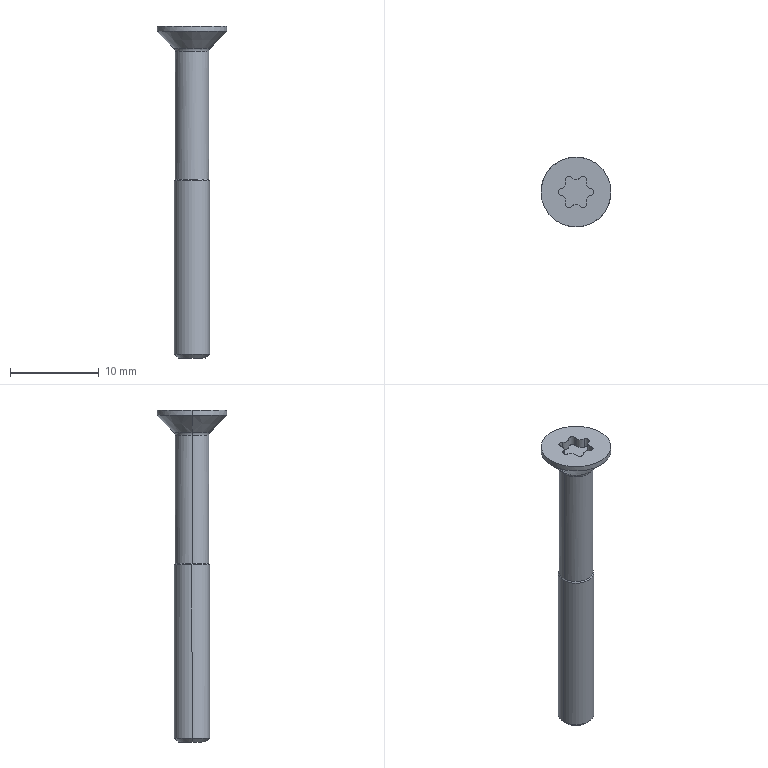Part | SolidWorks | features BaseBody 1 | 1 solid | 29 faces | box 7.9 x 7.9 x 37.5 mm | volume 495.827 mm3 | cylinder 18 | cone 6 | plane 3 | torus 2 | commonest cylinder face diameters 0.79 x6 1.383 x6 3.8 x2 4 x2 7.9 x2
STEP:
#1=CARTESIAN_POINT('',(-2.,0.,-37.071));
#2=VERTEX_POINT('',#1);
#3=CARTESIAN_POINT('',(2.,0.,-37.071));
#4=VERTEX_POINT('',#3);
#5=CARTESIAN_POINT('',(-2.,0.,-37.071));
#6=CARTESIAN_POINT('',(-2.,0.2618,-37.071));
#7=CARTESIAN_POINT('',(-1.948,0.5235,-37.071));
#8=CARTESIAN_POINT('',(-1.748,1.007,-37.07));
#9=CARTESIAN_POINT('',(-1.599,1.229,-37.071));
#10=CARTESIAN_POINT('',(-1.229,1.599,-37.071));
#11=CARTESIAN_POINT('',(-1.007,1.748,-37.071));
#12=CARTESIAN_POINT('',(-0.5235,1.948,-37.071));
#13=CARTESIAN_POINT('',(-0.2618,2.,-37.071));
#14=CARTESIAN_POINT('',(0.2618,2.,-37.071));
#15=CARTESIAN_POINT('',(0.5235,1.948,-37.071));
#16=CARTESIAN_POINT('',(1.007,1.748,-37.071));
#17=CARTESIAN_POINT('',(1.229,1.599,-37.071));
#18=CARTESIAN_POINT('',(1.599,1.229,-37.071));
#19=CARTESIAN_POINT('',(1.748,1.007,-37.071));
#20=CARTESIAN_POINT('',(1.948,0.5235,-37.071));
#21=CARTESIAN_POINT('',(2.,0.2618,-37.071));
#22=CARTESIAN_POINT('',(2.,0.,-37.071));
#23=B_SPLINE_CURVE_WITH_KNOTS('',3,(#5,#6,#7,#8,#9,#10,#11,#12,#13,#14,#15,#16,#17,#18,#19,#20,#21,#22),.UNSPECIFIED.,.F.,.F.,(4,2,2,2,2,2,2,2,4),(0.,0.125,0.25,0.375,0.5,0.625,0.75,0.875,1.),.UNSPECIFIED.);
#24=EDGE_CURVE('',#2,#4,#23,.T.);
#25=ORIENTED_EDGE('',*,*,#24,.F.);
#26=CARTESIAN_POINT('',(-2.,0.,-17.5));
#27=VERTEX_POINT('',#26);
#28=CARTESIAN_POINT('',(-2.,0.,-17.5));
#29=CARTESIAN_POINT('',(-2.,0.,-37.071));
#30=B_SPLINE_CURVE_WITH_KNOTS('',1,(#28,#29),.UNSPECIFIED.,.F.,.F.,(2,2),(0.,1.),.UNSPECIFIED.);
#31=EDGE_CURVE('',#27,#2,#30,.T.);
#32=ORIENTED_EDGE('',*,*,#31,.F.);
#33=CARTESIAN_POINT('',(2.,0.,-17.5));
#34=VERTEX_POINT('',#33);
#35=CARTESIAN_POINT('',(2.,0.,-17.5));
#36=CARTESIAN_POINT('',(2.,0.2618,-17.5));
#37=CARTESIAN_POINT('',(1.948,0.5235,-17.5));
#38=CARTESIAN_POINT('',(1.748,1.007,-17.5));
#39=CARTESIAN_POINT('',(1.599,1.229,-17.5));
#40=CARTESIAN_POINT('',(1.229,1.599,-17.5));
#41=CARTESIAN_POINT('',(1.007,1.748,-17.5));
#42=CARTESIAN_POINT('',(0.5235,1.948,-17.5));
#43=CARTESIAN_POINT('',(0.2618,2.,-17.5));
#44=CARTESIAN_POINT('',(-0.2618,2.,-17.5));
#45=CARTESIAN_POINT('',(-0.5235,1.948,-17.5));
#46=CARTESIAN_POINT('',(-1.007,1.748,-17.5));
#47=CARTESIAN_POINT('',(-1.229,1.599,-17.5));
#48=CARTESIAN_POINT('',(-1.599,1.229,-17.5));
#49=CARTESIAN_POINT('',(-1.748,1.007,-17.5));
#50=CARTESIAN_POINT('',(-1.948,0.5235,-17.5));
#51=CARTESIAN_POINT('',(-2.,0.2618,-17.5));
#52=CARTESIAN_POINT('',(-2.,0.,-17.5));
#53=B_SPLINE_CURVE_WITH_KNOTS('',3,(#35,#36,#37,#38,#39,#40,#41,#42,#43,#44,#45,#46,#47,#48,#49,#50,#51,#52),.UNSPECIFIED.,.F.,.F.,(4,2,2,2,2,2,2,2,4),(0.,0.125,0.25,0.375,0.5,0.625,0.75,0.875,1.),.UNSPECIFIED.);
#54=EDGE_CURVE('',#34,#27,#53,.T.);
#55=ORIENTED_EDGE('',*,*,#54,.F.);
#56=CARTESIAN_POINT('',(2.,0.,-37.071));
#57=CARTESIAN_POINT('',(2.,0.,-17.5));
#58=B_SPLINE_CURVE_WITH_KNOTS('',1,(#56,#57),.UNSPECIFIED.,.F.,.F.,(2,2),(0.,1.),.UNSPECIFIED.);
#59=EDGE_CURVE('',#4,#34,#58,.T.);
#60=ORIENTED_EDGE('',*,*,#59,.F.);
#61=EDGE_LOOP('',(#25,#32,#55,#60));
#62=FACE_OUTER_BOUND('',#61,.T.);
#63=CARTESIAN_POINT('',(0.,0.,-37.5));
#64=DIRECTION('',(0.,0.,-1.));
#65=DIRECTION('',(-1.,0.,0.));
#66=AXIS2_PLACEMENT_3D('',#63,#64,#65);
#67=CYLINDRICAL_SURFACE('',#66,2.);
#68=ADVANCED_FACE('',(#62),#67,.T.);
#69=CARTESIAN_POINT('',(-2.,0.,-17.5));
#70=CARTESIAN_POINT('',(-2.,-0.2618,-17.5));
#71=CARTESIAN_POINT('',(-1.948,-0.5235,-17.5));
#72=CARTESIAN_POINT('',(-1.748,-1.007,-17.5));
#73=CARTESIAN_POINT('',(-1.599,-1.229,-17.5));
#74=CARTESIAN_POINT('',(-1.229,-1.599,-17.5));
#75=CARTESIAN_POINT('',(-1.007,-1.748,-17.5));
#76=CARTESIAN_POINT('',(-0.5235,-1.948,-17.5));
#77=CARTESIAN_POINT('',(-0.2618,-2.,-17.5));
#78=CARTESIAN_POINT('',(0.2618,-2.,-17.5));
#79=CARTESIAN_POINT('',(0.5235,-1.948,-17.5));
#80=CARTESIAN_POINT('',(1.007,-1.748,-17.5));
#81=CARTESIAN_POINT('',(1.229,-1.599,-17.5));
#82=CARTESIAN_POINT('',(1.599,-1.229,-17.5));
#83=CARTESIAN_POINT('',(1.748,-1.007,-17.5));
#84=CARTESIAN_POINT('',(1.948,-0.5235,-17.5));
#85=CARTESIAN_POINT('',(2.,-0.2618,-17.5));
#86=CARTESIAN_POINT('',(2.,0.,-17.5));
#87=B_SPLINE_CURVE_WITH_KNOTS('',3,(#69,#70,#71,#72,#73,#74,#75,#76,#77,#78,#79,#80,#81,#82,#83,#84,#85,#86),.UNSPECIFIED.,.F.,.F.,(4,2,2,2,2,2,2,2,4),(0.,0.125,0.25,0.375,0.5,0.625,0.75,0.875,1.),.UNSPECIFIED.);
#88=EDGE_CURVE('',#27,#34,#87,.T.);
#89=ORIENTED_EDGE('',*,*,#88,.F.);
#90=ORIENTED_EDGE('',*,*,#31,.T.);
#91=CARTESIAN_POINT('',(2.,0.,-37.071));
#92=CARTESIAN_POINT('',(2.,-0.2618,-37.071));
#93=CARTESIAN_POINT('',(1.948,-0.5235,-37.071));
#94=CARTESIAN_POINT('',(1.748,-1.007,-37.07));
#95=CARTESIAN_POINT('',(1.599,-1.229,-37.071));
#96=CARTESIAN_POINT('',(1.229,-1.599,-37.071));
#97=CARTESIAN_POINT('',(1.007,-1.748,-37.071));
#98=CARTESIAN_POINT('',(0.5235,-1.948,-37.071));
#99=CARTESIAN_POINT('',(0.2618,-2.,-37.071));
#100=CARTESIAN_POINT('',(-0.2618,-2.,-37.071));
#101=CARTESIAN_POINT('',(-0.5235,-1.948,-37.071));
#102=CARTESIAN_POINT('',(-1.007,-1.748,-37.071));
#103=CARTESIAN_POINT('',(-1.229,-1.599,-37.071));
#104=CARTESIAN_POINT('',(-1.599,-1.229,-37.071));
#105=CARTESIAN_POINT('',(-1.748,-1.007,-37.071));
#106=CARTESIAN_POINT('',(-1.948,-0.5235,-37.071));
#107=CARTESIAN_POINT('',(-2.,-0.2618,-37.071));
#108=CARTESIAN_POINT('',(-2.,0.,-37.071));
#109=B_SPLINE_CURVE_WITH_KNOTS('',3,(#91,#92,#93,#94,#95,#96,#97,#98,#99,#100,#101,#102,#103,#104,#105,#106,#107,#108),.UNSPECIFIED.,.F.,.F.,(4,2,2,2,2,2,2,2,4),(0.,0.125,0.25,0.375,0.5,0.625,0.75,0.875,1.),.UNSPECIFIED.);
#110=EDGE_CURVE('',#4,#2,#109,.T.);
#111=ORIENTED_EDGE('',*,*,#110,.F.);
#112=ORIENTED_EDGE('',*,*,#59,.T.);
#113=EDGE_LOOP('',(#89,#90,#111,#112));
#114=FACE_OUTER_BOUND('',#113,.T.);
#115=CARTESIAN_POINT('',(0.,0.,-37.5));
#116=DIRECTION('',(0.,0.,-1.));
#117=DIRECTION('',(1.,0.000000001,0.));
#118=AXIS2_PLACEMENT_3D('',#115,#116,#117);
#119=CYLINDRICAL_SURFACE('',#118,2.);
#120=ADVANCED_FACE('',(#114),#119,.T.);
#121=CARTESIAN_POINT('',(-1.9,0.,-17.327));
#122=VERTEX_POINT('',#121);
#123=CARTESIAN_POINT('',(1.9,0.,-17.327));
#124=VERTEX_POINT('',#123);
#125=CARTESIAN_POINT('',(-1.9,0.,-17.327));
#126=CARTESIAN_POINT('',(-1.9,0.2487,-17.327));
#127=CARTESIAN_POINT('',(-1.851,0.4973,-17.327));
#128=CARTESIAN_POINT('',(-1.66,0.9569,-17.327));
#129=CARTESIAN_POINT('',(-1.519,1.168,-17.327));
#130=CARTESIAN_POINT('',(-1.168,1.519,-17.327));
#131=CARTESIAN_POINT('',(-0.9569,1.66,-17.327));
#132=CARTESIAN_POINT('',(-0.4973,1.851,-17.327));
#133=CARTESIAN_POINT('',(-0.2487,1.9,-17.327));
#134=CARTESIAN_POINT('',(0.2487,1.9,-17.327));
#135=CARTESIAN_POINT('',(0.4973,1.851,-17.327));
#136=CARTESIAN_POINT('',(0.9569,1.66,-17.327));
#137=CARTESIAN_POINT('',(1.168,1.519,-17.327));
#138=CARTESIAN_POINT('',(1.519,1.168,-17.327));
#139=CARTESIAN_POINT('',(1.66,0.9569,-17.327));
#140=CARTESIAN_POINT('',(1.851,0.4973,-17.327));
#141=CARTESIAN_POINT('',(1.9,0.2487,-17.327));
#142=CARTESIAN_POINT('',(1.9,0.,-17.327));
#143=B_SPLINE_CURVE_WITH_KNOTS('',3,(#125,#126,#127,#128,#129,#130,#131,#132,#133,#134,#135,#136,#137,#138,#139,#140,#141,#142),.UNSPECIFIED.,.F.,.F.,(4,2,2,2,2,2,2,2,4),(0.,0.125,0.25,0.375,0.5,0.625,0.75,0.875,1.),.UNSPECIFIED.);
#144=EDGE_CURVE('',#122,#124,#143,.T.);
#145=ORIENTED_EDGE('',*,*,#144,.F.);
#146=CARTESIAN_POINT('',(-1.9,0.,-2.857));
#147=VERTEX_POINT('',#146);
#148=CARTESIAN_POINT('',(-1.9,0.,-2.857));
#149=CARTESIAN_POINT('',(-1.9,0.,-17.327));
#150=B_SPLINE_CURVE_WITH_KNOTS('',1,(#148,#149),.UNSPECIFIED.,.F.,.F.,(2,2),(0.,1.),.UNSPECIFIED.);
#151=EDGE_CURVE('',#147,#122,#150,.T.);
#152=ORIENTED_EDGE('',*,*,#151,.F.);
#153=CARTESIAN_POINT('',(1.9,0.,-2.857));
#154=VERTEX_POINT('',#153);
#155=CARTESIAN_POINT('',(1.9,0.,-2.857));
#156=CARTESIAN_POINT('',(1.9,0.2487,-2.857));
#157=CARTESIAN_POINT('',(1.851,0.4973,-2.857));
#158=CARTESIAN_POINT('',(1.66,0.9569,-2.857));
#159=CARTESIAN_POINT('',(1.519,1.168,-2.857));
#160=CARTESIAN_POINT('',(1.168,1.519,-2.857));
#161=CARTESIAN_POINT('',(0.9569,1.66,-2.857));
#162=CARTESIAN_POINT('',(0.4973,1.851,-2.857));
#163=CARTESIAN_POINT('',(0.2487,1.9,-2.857));
#164=CARTESIAN_POINT('',(-0.2487,1.9,-2.857));
#165=CARTESIAN_POINT('',(-0.4973,1.851,-2.857));
#166=CARTESIAN_POINT('',(-0.9569,1.66,-2.857));
#167=CARTESIAN_POINT('',(-1.168,1.519,-2.857));
#168=CARTESIAN_POINT('',(-1.519,1.168,-2.857));
#169=CARTESIAN_POINT('',(-1.66,0.9569,-2.857));
#170=CARTESIAN_POINT('',(-1.851,0.4973,-2.857));
#171=CARTESIAN_POINT('',(-1.9,0.2487,-2.857));
#172=CARTESIAN_POINT('',(-1.9,0.,-2.857));
#173=B_SPLINE_CURVE_WITH_KNOTS('',3,(#155,#156,#157,#158,#159,#160,#161,#162,#163,#164,#165,#166,#167,#168,#169,#170,#171,#172),.UNSPECIFIED.,.F.,.F.,(4,2,2,2,2,2,2,2,4),(0.,0.125,0.25,0.375,0.5,0.625,0.75,0.875,1.),.UNSPECIFIED.);
#174=EDGE_CURVE('',#154,#147,#173,.T.);
#175=ORIENTED_EDGE('',*,*,#174,.F.);
#176=CARTESIAN_POINT('',(1.9,0.,-17.327));
#177=CARTESIAN_POINT('',(1.9,0.,-2.857));
#178=B_SPLINE_CURVE_WITH_KNOTS('',1,(#176,#177),.UNSPECIFIED.,.F.,.F.,(2,2),(0.,1.),.UNSPECIFIED.);
#179=EDGE_CURVE('',#124,#154,#178,.T.);
#180=ORIENTED_EDGE('',*,*,#179,.F.);
#181=EDGE_LOOP('',(#145,#152,#175,#180));
#182=FACE_OUTER_BOUND('',#181,.T.);
#183=CARTESIAN_POINT('',(0.,0.,-37.5));
#184=DIRECTION('',(0.,0.,-1.));
#185=DIRECTION('',(-1.,0.,0.));
#186=AXIS2_PLACEMENT_3D('',#183,#184,#185);
#187=CYLINDRICAL_SURFACE('',#186,1.9);
#188=ADVANCED_FACE('',(#182),#187,.T.);
#189=CARTESIAN_POINT('',(-1.9,0.,-2.857));
#190=CARTESIAN_POINT('',(-1.9,-0.2487,-2.857));
#191=CARTESIAN_POINT('',(-1.851,-0.4973,-2.857));
#192=CARTESIAN_POINT('',(-1.66,-0.9569,-2.857));
#193=CARTESIAN_POINT('',(-1.519,-1.168,-2.857));
#194=CARTESIAN_POINT('',(-1.168,-1.519,-2.857));
#195=CARTESIAN_POINT('',(-0.9569,-1.66,-2.857));
#196=CARTESIAN_POINT('',(-0.4973,-1.851,-2.857));
#197=CARTESIAN_POINT('',(-0.2487,-1.9,-2.857));
#198=CARTESIAN_POINT('',(0.2487,-1.9,-2.857));
#199=CARTESIAN_POINT('',(0.4973,-1.851,-2.857));
#200=CARTESIAN_POINT('',(0.9569,-1.66,-2.857));
#201=CARTESIAN_POINT('',(1.168,-1.519,-2.857));
#202=CARTESIAN_POINT('',(1.519,-1.168,-2.857));
#203=CARTESIAN_POINT('',(1.66,-0.9569,-2.857));
#204=CARTESIAN_POINT('',(1.851,-0.4973,-2.857));
#205=CARTESIAN_POINT('',(1.9,-0.2487,-2.857));
#206=CARTESIAN_POINT('',(1.9,0.,-2.857));
#207=B_SPLINE_CURVE_WITH_KNOTS('',3,(#189,#190,#191,#192,#193,#194,#195,#196,#197,#198,#199,#200,#201,#202,#203,#204,#205,#206),.UNSPECIFIED.,.F.,.F.,(4,2,2,2,2,2,2,2,4),(0.,0.125,0.25,0.375,0.5,0.625,0.75,0.875,1.),.UNSPECIFIED.);
#208=EDGE_CURVE('',#147,#154,#207,.T.);
#209=ORIENTED_EDGE('',*,*,#208,.F.);
#210=ORIENTED_EDGE('',*,*,#151,.T.);
#211=CARTESIAN_POINT('',(1.9,0.,-17.327));
#212=CARTESIAN_POINT('',(1.9,-0.2487,-17.327));
#213=CARTESIAN_POINT('',(1.851,-0.4973,-17.327));
#214=CARTESIAN_POINT('',(1.66,-0.9569,-17.327));
#215=CARTESIAN_POINT('',(1.519,-1.168,-17.327));
#216=CARTESIAN_POINT('',(1.168,-1.519,-17.327));
#217=CARTESIAN_POINT('',(0.9569,-1.66,-17.327));
#218=CARTESIAN_POINT('',(0.4973,-1.851,-17.327));
#219=CARTESIAN_POINT('',(0.2487,-1.9,-17.327));
#220=CARTESIAN_POINT('',(-0.2487,-1.9,-17.327));
#221=CARTESIAN_POINT('',(-0.4973,-1.851,-17.327));
#222=CARTESIAN_POINT('',(-0.9569,-1.66,-17.327));
#223=CARTESIAN_POINT('',(-1.168,-1.519,-17.327));
#224=CARTESIAN_POINT('',(-1.519,-1.168,-17.327));
#225=CARTESIAN_POINT('',(-1.66,-0.9569,-17.327));
#226=CARTESIAN_POINT('',(-1.851,-0.4973,-17.327));
#227=CARTESIAN_POINT('',(-1.9,-0.2487,-17.327));
#228=CARTESIAN_POINT('',(-1.9,0.,-17.327));
#229=B_SPLINE_CURVE_WITH_KNOTS('',3,(#211,#212,#213,#214,#215,#216,#217,#218,#219,#220,#221,#222,#223,#224,#225,#226,#227,#228),.UNSPECIFIED.,.F.,.F.,(4,2,2,2,2,2,2,2,4),(0.,0.125,0.25,0.375,0.5,0.625,0.75,0.875,1.),.UNSPECIFIED.);
#230=EDGE_CURVE('',#124,#122,#229,.T.);
#231=ORIENTED_EDGE('',*,*,#230,.F.);
#232=ORIENTED_EDGE('',*,*,#179,.T.);
#233=EDGE_LOOP('',(#209,#210,#231,#232));
#234=FACE_OUTER_BOUND('',#233,.T.);
#235=CARTESIAN_POINT('',(0.,0.,-37.5));
#236=DIRECTION('',(0.,0.,-1.));
#237=DIRECTION('',(1.,0.,0.));
#238=AXIS2_PLACEMENT_3D('',#235,#236,#237);
#239=CYLINDRICAL_SURFACE('',#238,1.9);
#240=ADVANCED_FACE('',(#234),#239,.T.);
#241=ORIENTED_EDGE('',*,*,#174,.T.);
#242=CARTESIAN_POINT('',(-2.046,0.,-2.504));
#243=VERTEX_POINT('',#242);
#244=CARTESIAN_POINT('',(-2.046,0.,-2.504));
#245=CARTESIAN_POINT('',(-1.954,0.,-2.596));
#246=CARTESIAN_POINT('',(-1.9,0.,-2.726));
#247=CARTESIAN_POINT('',(-1.9,0.,-2.857));
#248=B_SPLINE_CURVE_WITH_KNOTS('',3,(#244,#245,#246,#247),.UNSPECIFIED.,.F.,.F.,(4,4),(0.,1.),.UNSPECIFIED.);
#249=EDGE_CURVE('',#243,#147,#248,.T.);
#250=ORIENTED_EDGE('',*,*,#249,.F.);
#251=CARTESIAN_POINT('',(2.046,0.,-2.504));
#252=VERTEX_POINT('',#251);
#253=CARTESIAN_POINT('',(2.046,0.,-2.504));
#254=CARTESIAN_POINT('',(2.046,0.2679,-2.504));
#255=CARTESIAN_POINT('',(1.993,0.5357,-2.504));
#256=CARTESIAN_POINT('',(1.788,1.031,-2.504));
#257=CARTESIAN_POINT('',(1.636,1.258,-2.504));
#258=CARTESIAN_POINT('',(1.258,1.636,-2.504));
#259=CARTESIAN_POINT('',(1.031,1.788,-2.504));
#260=CARTESIAN_POINT('',(0.5357,1.993,-2.504));
#261=CARTESIAN_POINT('',(0.2679,2.046,-2.504));
#262=CARTESIAN_POINT('',(-0.2679,2.046,-2.504));
#263=CARTESIAN_POINT('',(-0.5357,1.993,-2.504));
#264=CARTESIAN_POINT('',(-1.031,1.788,-2.504));
#265=CARTESIAN_POINT('',(-1.258,1.636,-2.504));
#266=CARTESIAN_POINT('',(-1.636,1.258,-2.504));
#267=CARTESIAN_POINT('',(-1.788,1.031,-2.504));
#268=CARTESIAN_POINT('',(-1.993,0.5357,-2.504));
#269=CARTESIAN_POINT('',(-2.046,0.2679,-2.504));
#270=CARTESIAN_POINT('',(-2.046,0.,-2.504));
#271=B_SPLINE_CURVE_WITH_KNOTS('',3,(#253,#254,#255,#256,#257,#258,#259,#260,#261,#262,#263,#264,#265,#266,#267,#268,#269,#270),.UNSPECIFIED.,.F.,.F.,(4,2,2,2,2,2,2,2,4),(0.,0.125,0.25,0.375,0.5,0.625,0.75,0.875,1.),.UNSPECIFIED.);
#272=EDGE_CURVE('',#252,#243,#271,.T.);
#273=ORIENTED_EDGE('',*,*,#272,.F.);
#274=CARTESIAN_POINT('',(1.9,0.,-2.857));
#275=CARTESIAN_POINT('',(1.9,0.000000002,-2.726));
#276=CARTESIAN_POINT('',(1.954,0.000000001,-2.596));
#277=CARTESIAN_POINT('',(2.046,0.,-2.504));
#278=B_SPLINE_CURVE_WITH_KNOTS('',3,(#274,#275,#276,#277),.UNSPECIFIED.,.F.,.F.,(4,4),(0.,1.),.UNSPECIFIED.);
#279=EDGE_CURVE('',#154,#252,#278,.T.);
#280=ORIENTED_EDGE('',*,*,#279,.F.);
#281=EDGE_LOOP('',(#241,#250,#273,#280));
#282=FACE_OUTER_BOUND('',#281,.T.);
#283=CARTESIAN_POINT('',(0.,0.,-2.857));
#284=DIRECTION('',(0.,0.,-1.));
#285=DIRECTION('',(-1.,0.,0.));
#286=AXIS2_PLACEMENT_3D('',#283,#284,#285);
#287=TOROIDAL_SURFACE('',#286,2.4,0.5);
#288=ADVANCED_FACE('',(#282),#287,.F.);
#289=ORIENTED_EDGE('',*,*,#208,.T.);
#290=ORIENTED_EDGE('',*,*,#279,.T.);
#291=CARTESIAN_POINT('',(-2.046,0.,-2.504));
#292=CARTESIAN_POINT('',(-2.046,-0.2679,-2.504));
#293=CARTESIAN_POINT('',(-1.993,-0.5357,-2.504));
#294=CARTESIAN_POINT('',(-1.788,-1.031,-2.504));
#295=CARTESIAN_POINT('',(-1.636,-1.258,-2.504));
#296=CARTESIAN_POINT('',(-1.258,-1.636,-2.504));
#297=CARTESIAN_POINT('',(-1.031,-1.788,-2.504));
#298=CARTESIAN_POINT('',(-0.5357,-1.993,-2.504));
#299=CARTESIAN_POINT('',(-0.2679,-2.046,-2.504));
#300=CARTESIAN_POINT('',(0.2679,-2.046,-2.504));
#301=CARTESIAN_POINT('',(0.5357,-1.993,-2.504));
#302=CARTESIAN_POINT('',(1.031,-1.788,-2.504));
#303=CARTESIAN_POINT('',(1.258,-1.636,-2.504));
#304=CARTESIAN_POINT('',(1.636,-1.258,-2.504));
#305=CARTESIAN_POINT('',(1.788,-1.031,-2.504));
#306=CARTESIAN_POINT('',(1.993,-0.5357,-2.504));
#307=CARTESIAN_POINT('',(2.046,-0.2679,-2.504));
#308=CARTESIAN_POINT('',(2.046,0.,-2.504));
#309=B_SPLINE_CURVE_WITH_KNOTS('',3,(#291,#292,#293,#294,#295,#296,#297,#298,#299,#300,#301,#302,#303,#304,#305,#306,#307,#308),.UNSPECIFIED.,.F.,.F.,(4,2,2,2,2,2,2,2,4),(0.,0.125,0.25,0.375,0.5,0.625,0.75,0.875,1.),.UNSPECIFIED.);
#310=EDGE_CURVE('',#243,#252,#309,.T.);
#311=ORIENTED_EDGE('',*,*,#310,.F.);
#312=ORIENTED_EDGE('',*,*,#249,.T.);
#313=EDGE_LOOP('',(#289,#290,#311,#312));
#314=FACE_OUTER_BOUND('',#313,.T.);
#315=CARTESIAN_POINT('',(0.,0.,-2.857));
#316=DIRECTION('',(0.,0.,-1.));
#317=DIRECTION('',(1.,0.000000001,0.));
#318=AXIS2_PLACEMENT_3D('',#315,#316,#317);
#319=TOROIDAL_SURFACE('',#318,2.4,0.5);
#320=ADVANCED_FACE('',(#314),#319,.F.);
#321=CARTESIAN_POINT('',(-3.95,0.,-0.6));
#322=VERTEX_POINT('',#321);
#323=CARTESIAN_POINT('',(3.95,0.,-0.6));
#324=VERTEX_POINT('',#323);
#325=CARTESIAN_POINT('',(-3.95,0.,-0.6));
#326=CARTESIAN_POINT('',(-3.95,0.5171,-0.6));
#327=CARTESIAN_POINT('',(-3.847,1.034,-0.6));
#328=CARTESIAN_POINT('',(-3.451,1.989,-0.6));
#329=CARTESIAN_POINT('',(-3.159,2.427,-0.6));
#330=CARTESIAN_POINT('',(-2.427,3.159,-0.6));
#331=CARTESIAN_POINT('',(-1.989,3.451,-0.6));
#332=CARTESIAN_POINT('',(-1.034,3.847,-0.6));
#333=CARTESIAN_POINT('',(-0.5171,3.95,-0.6));
#334=CARTESIAN_POINT('',(0.5171,3.95,-0.6));
#335=CARTESIAN_POINT('',(1.034,3.847,-0.6));
#336=CARTESIAN_POINT('',(1.989,3.451,-0.6));
#337=CARTESIAN_POINT('',(2.427,3.159,-0.6));
#338=CARTESIAN_POINT('',(3.159,2.427,-0.6));
#339=CARTESIAN_POINT('',(3.451,1.989,-0.6));
#340=CARTESIAN_POINT('',(3.847,1.034,-0.6));
#341=CARTESIAN_POINT('',(3.95,0.5171,-0.6));
#342=CARTESIAN_POINT('',(3.95,0.,-0.6));
#343=B_SPLINE_CURVE_WITH_KNOTS('',3,(#325,#326,#327,#328,#329,#330,#331,#332,#333,#334,#335,#336,#337,#338,#339,#340,#341,#342),.UNSPECIFIED.,.F.,.F.,(4,2,2,2,2,2,2,2,4),(0.,0.125,0.25,0.375,0.5,0.625,0.75,0.875,1.),.UNSPECIFIED.);
#344=EDGE_CURVE('',#322,#324,#343,.T.);
#345=ORIENTED_EDGE('',*,*,#344,.F.);
#346=CARTESIAN_POINT('',(-3.95,0.,0.));
#347=VERTEX_POINT('',#346);
#348=CARTESIAN_POINT('',(-3.95,0.,0.));
#349=CARTESIAN_POINT('',(-3.95,0.,-0.6));
#350=B_SPLINE_CURVE_WITH_KNOTS('',1,(#348,#349),.UNSPECIFIED.,.F.,.F.,(2,2),(0.,1.),.UNSPECIFIED.);
#351=EDGE_CURVE('',#347,#322,#350,.T.);
#352=ORIENTED_EDGE('',*,*,#351,.F.);
#353=CARTESIAN_POINT('',(3.95,0.,0.));
#354=VERTEX_POINT('',#353);
#355=CARTESIAN_POINT('',(3.95,0.,0.));
#356=CARTESIAN_POINT('',(3.95,0.5236,0.));
#357=CARTESIAN_POINT('',(3.85,1.028,0.));
#358=CARTESIAN_POINT('',(3.449,1.995,0.));
#359=CARTESIAN_POINT('',(3.163,2.423,0.));
#360=CARTESIAN_POINT('',(2.423,3.163,0.));
#361=CARTESIAN_POINT('',(1.995,3.449,0.));
#362=CARTESIAN_POINT('',(1.028,3.85,0.));
#363=CARTESIAN_POINT('',(0.5235,3.95,0.));
#364=CARTESIAN_POINT('',(-0.5235,3.95,0.));
#365=CARTESIAN_POINT('',(-1.028,3.85,0.));
#366=CARTESIAN_POINT('',(-1.995,3.449,0.));
#367=CARTESIAN_POINT('',(-2.423,3.163,0.));
#368=CARTESIAN_POINT('',(-3.163,2.423,0.));
#369=CARTESIAN_POINT('',(-3.449,1.995,0.));
#370=CARTESIAN_POINT('',(-3.85,1.028,0.));
#371=CARTESIAN_POINT('',(-3.95,0.524,0.));
#372=CARTESIAN_POINT('',(-3.95,0.,0.));
#373=B_SPLINE_CURVE_WITH_KNOTS('',3,(#355,#356,#357,#358,#359,#360,#361,#362,#363,#364,#365,#366,#367,#368,#369,#370,#371,#372),.UNSPECIFIED.,.F.,.F.,(4,2,2,2,2,2,2,2,4),(0.,0.125,0.25,0.375,0.5,0.625,0.75,0.875,1.),.UNSPECIFIED.);
#374=EDGE_CURVE('',#354,#347,#373,.T.);
#375=ORIENTED_EDGE('',*,*,#374,.F.);
#376=CARTESIAN_POINT('',(3.95,0.,-0.6));
#377=CARTESIAN_POINT('',(3.95,0.,0.));
#378=B_SPLINE_CURVE_WITH_KNOTS('',1,(#376,#377),.UNSPECIFIED.,.F.,.F.,(2,2),(0.,1.),.UNSPECIFIED.);
#379=EDGE_CURVE('',#324,#354,#378,.T.);
#380=ORIENTED_EDGE('',*,*,#379,.F.);
#381=EDGE_LOOP('',(#345,#352,#375,#380));
#382=FACE_OUTER_BOUND('',#381,.T.);
#383=CARTESIAN_POINT('',(0.,0.,-37.5));
#384=DIRECTION('',(0.,0.,-1.));
#385=DIRECTION('',(-1.,0.,0.));
#386=AXIS2_PLACEMENT_3D('',#383,#384,#385);
#387=CYLINDRICAL_SURFACE('',#386,3.95);
#388=ADVANCED_FACE('',(#382),#387,.T.);
#389=CARTESIAN_POINT('',(-3.95,0.,0.));
#390=CARTESIAN_POINT('',(-3.95,-0.5236,0.));
#391=CARTESIAN_POINT('',(-3.85,-1.028,0.));
#392=CARTESIAN_POINT('',(-3.449,-1.995,0.));
#393=CARTESIAN_POINT('',(-3.163,-2.423,0.));
#394=CARTESIAN_POINT('',(-2.423,-3.163,0.));
#395=CARTESIAN_POINT('',(-1.995,-3.449,0.));
#396=CARTESIAN_POINT('',(-1.028,-3.85,0.));
#397=CARTESIAN_POINT('',(-0.5235,-3.95,0.));
#398=CARTESIAN_POINT('',(0.5235,-3.95,0.));
#399=CARTESIAN_POINT('',(1.028,-3.85,0.));
#400=CARTESIAN_POINT('',(1.995,-3.449,0.));
#401=CARTESIAN_POINT('',(2.423,-3.163,0.));
#402=CARTESIAN_POINT('',(3.163,-2.423,0.));
#403=CARTESIAN_POINT('',(3.449,-1.995,0.));
#404=CARTESIAN_POINT('',(3.85,-1.028,0.));
#405=CARTESIAN_POINT('',(3.95,-0.524,0.));
#406=CARTESIAN_POINT('',(3.95,0.,0.));
#407=B_SPLINE_CURVE_WITH_KNOTS('',3,(#389,#390,#391,#392,#393,#394,#395,#396,#397,#398,#399,#400,#401,#402,#403,#404,#405,#406),.UNSPECIFIED.,.F.,.F.,(4,2,2,2,2,2,2,2,4),(0.,0.125,0.25,0.375,0.5,0.625,0.75,0.875,1.),.UNSPECIFIED.);
#408=EDGE_CURVE('',#347,#354,#407,.T.);
#409=ORIENTED_EDGE('',*,*,#408,.F.);
#410=ORIENTED_EDGE('',*,*,#351,.T.);
#411=CARTESIAN_POINT('',(3.95,0.,-0.6));
#412=CARTESIAN_POINT('',(3.95,-0.5171,-0.6));
#413=CARTESIAN_POINT('',(3.847,-1.034,-0.6));
#414=CARTESIAN_POINT('',(3.451,-1.989,-0.6));
#415=CARTESIAN_POINT('',(3.159,-2.427,-0.6));
#416=CARTESIAN_POINT('',(2.427,-3.159,-0.6));
#417=CARTESIAN_POINT('',(1.989,-3.451,-0.6));
#418=CARTESIAN_POINT('',(1.034,-3.847,-0.6));
#419=CARTESIAN_POINT('',(0.5171,-3.95,-0.6));
#420=CARTESIAN_POINT('',(-0.5171,-3.95,-0.6));
#421=CARTESIAN_POINT('',(-1.034,-3.847,-0.6));
#422=CARTESIAN_POINT('',(-1.989,-3.451,-0.6));
#423=CARTESIAN_POINT('',(-2.427,-3.159,-0.6));
#424=CARTESIAN_POINT('',(-3.159,-2.427,-0.6));
#425=CARTESIAN_POINT('',(-3.451,-1.989,-0.6));
#426=CARTESIAN_POINT('',(-3.847,-1.034,-0.6));
#427=CARTESIAN_POINT('',(-3.95,-0.5171,-0.6));
#428=CARTESIAN_POINT('',(-3.95,0.,-0.6));
#429=B_SPLINE_CURVE_WITH_KNOTS('',3,(#411,#412,#413,#414,#415,#416,#417,#418,#419,#420,#421,#422,#423,#424,#425,#426,#427,#428),.UNSPECIFIED.,.F.,.F.,(4,2,2,2,2,2,2,2,4),(0.,0.125,0.25,0.375,0.5,0.625,0.75,0.875,1.),.UNSPECIFIED.);
#430=EDGE_CURVE('',#324,#322,#429,.T.);
#431=ORIENTED_EDGE('',*,*,#430,.F.);
#432=ORIENTED_EDGE('',*,*,#379,.T.);
#433=EDGE_LOOP('',(#409,#410,#431,#432));
#434=FACE_OUTER_BOUND('',#433,.T.);
#435=CARTESIAN_POINT('',(0.,0.,-37.5));
#436=DIRECTION('',(0.,0.,-1.));
#437=DIRECTION('',(1.,0.,0.));
#438=AXIS2_PLACEMENT_3D('',#435,#436,#437);
#439=CYLINDRICAL_SURFACE('',#438,3.95);
#440=ADVANCED_FACE('',(#434),#439,.T.);
#441=ORIENTED_EDGE('',*,*,#24,.T.);
#442=CARTESIAN_POINT('',(1.571,0.,-37.5));
#443=VERTEX_POINT('',#442);
#444=CARTESIAN_POINT('',(1.571,0.,-37.5));
#445=CARTESIAN_POINT('',(2.,0.,-37.071));
#446=B_SPLINE_CURVE_WITH_KNOTS('',1,(#444,#445),.UNSPECIFIED.,.F.,.F.,(2,2),(0.,1.),.UNSPECIFIED.);
#447=EDGE_CURVE('',#443,#4,#446,.T.);
#448=ORIENTED_EDGE('',*,*,#447,.F.);
#449=CARTESIAN_POINT('',(-1.571,0.,-37.5));
#450=VERTEX_POINT('',#449);
#451=CARTESIAN_POINT('',(-1.571,0.,-37.5));
#452=CARTESIAN_POINT('',(-1.571,0.2081,-37.5));
#453=CARTESIAN_POINT('',(-1.53,0.4089,-37.5));
#454=CARTESIAN_POINT('',(-1.371,0.7931,-37.5));
#455=CARTESIAN_POINT('',(-1.257,0.9634,-37.5));
#456=CARTESIAN_POINT('',(-0.9635,1.258,-37.5));
#457=CARTESIAN_POINT('',(-0.7931,1.371,-37.5));
#458=CARTESIAN_POINT('',(-0.4089,1.531,-37.5));
#459=CARTESIAN_POINT('',(-0.2079,1.57,-37.5));
#460=CARTESIAN_POINT('',(0.2079,1.571,-37.5));
#461=CARTESIAN_POINT('',(0.4089,1.53,-37.5));
#462=CARTESIAN_POINT('',(0.7931,1.371,-37.5));
#463=CARTESIAN_POINT('',(0.9634,1.257,-37.5));
#464=CARTESIAN_POINT('',(1.258,0.9635,-37.5));
#465=CARTESIAN_POINT('',(1.371,0.7932,-37.5));
#466=CARTESIAN_POINT('',(1.531,0.4088,-37.5));
#467=CARTESIAN_POINT('',(1.571,0.2084,-37.5));
#468=CARTESIAN_POINT('',(1.571,0.,-37.5));
#469=B_SPLINE_CURVE_WITH_KNOTS('',3,(#451,#452,#453,#454,#455,#456,#457,#458,#459,#460,#461,#462,#463,#464,#465,#466,#467,#468),.UNSPECIFIED.,.F.,.F.,(4,2,2,2,2,2,2,2,4),(0.,0.125,0.25,0.375,0.5,0.625,0.75,0.875,1.),.UNSPECIFIED.);
#470=EDGE_CURVE('',#450,#443,#469,.T.);
#471=ORIENTED_EDGE('',*,*,#470,.F.);
#472=CARTESIAN_POINT('',(-2.,0.,-37.071));
#473=CARTESIAN_POINT('',(-1.571,0.,-37.5));
#474=B_SPLINE_CURVE_WITH_KNOTS('',1,(#472,#473),.UNSPECIFIED.,.F.,.F.,(2,2),(0.,1.),.UNSPECIFIED.);
#475=EDGE_CURVE('',#2,#450,#474,.T.);
#476=ORIENTED_EDGE('',*,*,#475,.F.);
#477=EDGE_LOOP('',(#441,#448,#471,#476));
#478=FACE_OUTER_BOUND('',#477,.T.);
#479=CARTESIAN_POINT('',(0.,0.,-37.071));
#480=DIRECTION('',(0.,0.,1.));
#481=DIRECTION('',(1.,0.,0.));
#482=AXIS2_PLACEMENT_3D('',#479,#480,#481);
#483=CONICAL_SURFACE('',#482,2.,0.7854);
#484=ADVANCED_FACE('',(#478),#483,.T.);
#485=CARTESIAN_POINT('',(1.571,0.,-37.5));
#486=CARTESIAN_POINT('',(1.571,-0.2081,-37.5));
#487=CARTESIAN_POINT('',(1.53,-0.4089,-37.5));
#488=CARTESIAN_POINT('',(1.371,-0.7931,-37.5));
#489=CARTESIAN_POINT('',(1.257,-0.9634,-37.5));
#490=CARTESIAN_POINT('',(0.9635,-1.258,-37.5));
#491=CARTESIAN_POINT('',(0.7931,-1.371,-37.5));
#492=CARTESIAN_POINT('',(0.4089,-1.531,-37.5));
#493=CARTESIAN_POINT('',(0.2079,-1.57,-37.5));
#494=CARTESIAN_POINT('',(-0.2079,-1.571,-37.5));
#495=CARTESIAN_POINT('',(-0.4089,-1.53,-37.5));
#496=CARTESIAN_POINT('',(-0.7931,-1.371,-37.5));
#497=CARTESIAN_POINT('',(-0.9634,-1.257,-37.5));
#498=CARTESIAN_POINT('',(-1.258,-0.9635,-37.5));
#499=CARTESIAN_POINT('',(-1.371,-0.7932,-37.5));
#500=CARTESIAN_POINT('',(-1.531,-0.4088,-37.5));
#501=CARTESIAN_POINT('',(-1.571,-0.2084,-37.5));
#502=CARTESIAN_POINT('',(-1.571,0.,-37.5));
#503=B_SPLINE_CURVE_WITH_KNOTS('',3,(#485,#486,#487,#488,#489,#490,#491,#492,#493,#494,#495,#496,#497,#498,#499,#500,#501,#502),.UNSPECIFIED.,.F.,.F.,(4,2,2,2,2,2,2,2,4),(0.,0.125,0.25,0.375,0.5,0.625,0.75,0.875,1.),.UNSPECIFIED.);
#504=EDGE_CURVE('',#443,#450,#503,.T.);
#505=ORIENTED_EDGE('',*,*,#504,.F.);
#506=ORIENTED_EDGE('',*,*,#447,.T.);
#507=ORIENTED_EDGE('',*,*,#110,.T.);
#508=ORIENTED_EDGE('',*,*,#475,.T.);
#509=EDGE_LOOP('',(#505,#506,#507,#508));
#510=FACE_OUTER_BOUND('',#509,.T.);
#511=CARTESIAN_POINT('',(0.,0.,-37.071));
#512=DIRECTION('',(0.,0.,1.));
#513=DIRECTION('',(-1.,0.,0.));
#514=AXIS2_PLACEMENT_3D('',#511,#512,#513);
#515=CONICAL_SURFACE('',#514,2.,0.7854);
#516=ADVANCED_FACE('',(#510),#515,.T.);
#517=ORIENTED_EDGE('',*,*,#54,.T.);
#518=CARTESIAN_POINT('',(-1.9,0.,-17.327));
#519=CARTESIAN_POINT('',(-2.,0.,-17.5));
#520=B_SPLINE_CURVE_WITH_KNOTS('',1,(#518,#519),.UNSPECIFIED.,.F.,.F.,(2,2),(0.,1.),.UNSPECIFIED.);
#521=EDGE_CURVE('',#122,#27,#520,.T.);
#522=ORIENTED_EDGE('',*,*,#521,.F.);
#523=ORIENTED_EDGE('',*,*,#144,.T.);
#524=CARTESIAN_POINT('',(2.,0.,-17.5));
#525=CARTESIAN_POINT('',(1.9,0.,-17.327));
#526=B_SPLINE_CURVE_WITH_KNOTS('',1,(#524,#525),.UNSPECIFIED.,.F.,.F.,(2,2),(0.,1.),.UNSPECIFIED.);
#527=EDGE_CURVE('',#34,#124,#526,.T.);
#528=ORIENTED_EDGE('',*,*,#527,.F.);
#529=EDGE_LOOP('',(#517,#522,#523,#528));
#530=FACE_OUTER_BOUND('',#529,.T.);
#531=CARTESIAN_POINT('',(0.,0.,-17.327));
#532=DIRECTION('',(0.,0.,-1.));
#533=DIRECTION('',(-1.,0.,0.));
#534=AXIS2_PLACEMENT_3D('',#531,#532,#533);
#535=CONICAL_SURFACE('',#534,1.9,0.5236);
#536=ADVANCED_FACE('',(#530),#535,.T.);
#537=ORIENTED_EDGE('',*,*,#88,.T.);
#538=ORIENTED_EDGE('',*,*,#527,.T.);
#539=ORIENTED_EDGE('',*,*,#230,.T.);
#540=ORIENTED_EDGE('',*,*,#521,.T.);
#541=EDGE_LOOP('',(#537,#538,#539,#540));
#542=FACE_OUTER_BOUND('',#541,.T.);
#543=CARTESIAN_POINT('',(0.,0.,-17.327));
#544=DIRECTION('',(0.,0.,-1.));
#545=DIRECTION('',(1.,0.,0.));
#546=AXIS2_PLACEMENT_3D('',#543,#544,#545);
#547=CONICAL_SURFACE('',#546,1.9,0.5236);
#548=ADVANCED_FACE('',(#542),#547,.T.);
#549=ORIENTED_EDGE('',*,*,#344,.T.);
#550=CARTESIAN_POINT('',(2.046,0.,-2.504));
#551=CARTESIAN_POINT('',(3.95,0.,-0.6));
#552=B_SPLINE_CURVE_WITH_KNOTS('',1,(#550,#551),.UNSPECIFIED.,.F.,.F.,(2,2),(0.,1.),.UNSPECIFIED.);
#553=EDGE_CURVE('',#252,#324,#552,.T.);
#554=ORIENTED_EDGE('',*,*,#553,.F.);
#555=ORIENTED_EDGE('',*,*,#272,.T.);
#556=CARTESIAN_POINT('',(-3.95,0.,-0.6));
#557=CARTESIAN_POINT('',(-2.046,0.,-2.504));
#558=B_SPLINE_CURVE_WITH_KNOTS('',1,(#556,#557),.UNSPECIFIED.,.F.,.F.,(2,2),(0.,1.),.UNSPECIFIED.);
#559=EDGE_CURVE('',#322,#243,#558,.T.);
#560=ORIENTED_EDGE('',*,*,#559,.F.);
#561=EDGE_LOOP('',(#549,#554,#555,#560));
#562=FACE_OUTER_BOUND('',#561,.T.);
#563=CARTESIAN_POINT('',(0.,0.,-0.6));
#564=DIRECTION('',(0.,0.,1.));
#565=DIRECTION('',(1.,0.,0.));
#566=AXIS2_PLACEMENT_3D('',#563,#564,#565);
#567=CONICAL_SURFACE('',#566,3.95,0.7854);
#568=ADVANCED_FACE('',(#562),#567,.T.);
#569=ORIENTED_EDGE('',*,*,#310,.T.);
#570=ORIENTED_EDGE('',*,*,#553,.T.);
#571=ORIENTED_EDGE('',*,*,#430,.T.);
#572=ORIENTED_EDGE('',*,*,#559,.T.);
#573=EDGE_LOOP('',(#569,#570,#571,#572));
#574=FACE_OUTER_BOUND('',#573,.T.);
#575=CARTESIAN_POINT('',(0.,0.,-0.6));
#576=DIRECTION('',(0.,0.,1.));
#577=DIRECTION('',(-1.,0.,0.));
#578=AXIS2_PLACEMENT_3D('',#575,#576,#577);
#579=CONICAL_SURFACE('',#578,3.95,0.7854);
#580=ADVANCED_FACE('',(#574),#579,.T.);
#581=CARTESIAN_POINT('',(-1.671,0.3843,-1.1));
#582=VERTEX_POINT('',#581);
#583=CARTESIAN_POINT('',(-1.168,1.255,-1.1));
#584=VERTEX_POINT('',#583);
#585=CARTESIAN_POINT('',(-1.671,0.3843,-1.1));
#586=CARTESIAN_POINT('',(-1.489,0.4276,-1.1));
#587=CARTESIAN_POINT('',(-1.326,0.5488,-1.1));
#588=CARTESIAN_POINT('',(-1.138,0.8738,-1.1));
#589=CARTESIAN_POINT('',(-1.115,1.075,-1.1));
#590=CARTESIAN_POINT('',(-1.168,1.255,-1.1));
#591=B_SPLINE_CURVE_WITH_KNOTS('',3,(#585,#586,#587,#588,#589,#590),.UNSPECIFIED.,.F.,.F.,(4,2,4),(0.,0.5,1.),.UNSPECIFIED.);
#592=EDGE_CURVE('',#582,#584,#591,.T.);
#593=ORIENTED_EDGE('',*,*,#592,.F.);
#594=CARTESIAN_POINT('',(-1.671,-0.3843,-1.1));
#595=VERTEX_POINT('',#594);
#596=CARTESIAN_POINT('',(-1.671,-0.3843,-1.1));
#597=CARTESIAN_POINT('',(-1.757,-0.364,-1.1));
#598=CARTESIAN_POINT('',(-1.835,-0.3141,-1.1));
#599=CARTESIAN_POINT('',(-1.944,-0.1759,-1.1));
#600=CARTESIAN_POINT('',(-1.975,-0.08808,-1.1));
#601=CARTESIAN_POINT('',(-1.975,0.08808,-1.1));
#602=CARTESIAN_POINT('',(-1.944,0.1759,-1.1));
#603=CARTESIAN_POINT('',(-1.835,0.3141,-1.1));
#604=CARTESIAN_POINT('',(-1.757,0.364,-1.1));
#605=CARTESIAN_POINT('',(-1.671,0.3843,-1.1));
#606=B_SPLINE_CURVE_WITH_KNOTS('',3,(#596,#597,#598,#599,#600,#601,#602,#603,#604,#605),.UNSPECIFIED.,.F.,.F.,(4,2,2,2,4),(0.,0.25,0.5,0.75,1.),.UNSPECIFIED.);
#607=EDGE_CURVE('',#595,#582,#606,.T.);
#608=ORIENTED_EDGE('',*,*,#607,.F.);
#609=CARTESIAN_POINT('',(-1.168,-1.255,-1.1));
#610=VERTEX_POINT('',#609);
#611=CARTESIAN_POINT('',(-1.168,-1.255,-1.1));
#612=CARTESIAN_POINT('',(-1.115,-1.075,-1.1));
#613=CARTESIAN_POINT('',(-1.138,-0.8738,-1.1));
#614=CARTESIAN_POINT('',(-1.326,-0.5488,-1.1));
#615=CARTESIAN_POINT('',(-1.489,-0.4276,-1.1));
#616=CARTESIAN_POINT('',(-1.671,-0.3843,-1.1));
#617=B_SPLINE_CURVE_WITH_KNOTS('',3,(#611,#612,#613,#614,#615,#616),.UNSPECIFIED.,.F.,.F.,(4,2,4),(0.,0.5,1.),.UNSPECIFIED.);
#618=EDGE_CURVE('',#610,#595,#617,.T.);
#619=ORIENTED_EDGE('',*,*,#618,.F.);
#620=CARTESIAN_POINT('',(-0.5027,-1.639,-1.1));
#621=VERTEX_POINT('',#620);
#622=CARTESIAN_POINT('',(-0.5027,-1.639,-1.1));
#623=CARTESIAN_POINT('',(-0.5632,-1.703,-1.1));
#624=CARTESIAN_POINT('',(-0.6456,-1.746,-1.1));
#625=CARTESIAN_POINT('',(-0.8199,-1.772,-1.1));
#626=CARTESIAN_POINT('',(-0.9112,-1.754,-1.1));
#627=CARTESIAN_POINT('',(-1.064,-1.666,-1.1));
#628=CARTESIAN_POINT('',(-1.125,-1.596,-1.1));
#629=CARTESIAN_POINT('',(-1.19,-1.432,-1.1));
#630=CARTESIAN_POINT('',(-1.194,-1.339,-1.1));
#631=CARTESIAN_POINT('',(-1.168,-1.255,-1.1));
#632=B_SPLINE_CURVE_WITH_KNOTS('',3,(#622,#623,#624,#625,#626,#627,#628,#629,#630,#631),.UNSPECIFIED.,.F.,.F.,(4,2,2,2,4),(0.,0.25,0.5,0.75,1.),.UNSPECIFIED.);
#633=EDGE_CURVE('',#621,#610,#632,.T.);
#634=ORIENTED_EDGE('',*,*,#633,.F.);
#635=CARTESIAN_POINT('',(0.5027,-1.639,-1.1));
#636=VERTEX_POINT('',#635);
#637=CARTESIAN_POINT('',(0.5027,-1.639,-1.1));
#638=CARTESIAN_POINT('',(0.3739,-1.503,-1.1));
#639=CARTESIAN_POINT('',(0.1876,-1.423,-1.1));
#640=CARTESIAN_POINT('',(-0.1876,-1.423,-1.1));
#641=CARTESIAN_POINT('',(-0.3739,-1.503,-1.1));
#642=CARTESIAN_POINT('',(-0.5027,-1.639,-1.1));
#643=B_SPLINE_CURVE_WITH_KNOTS('',3,(#637,#638,#639,#640,#641,#642),.UNSPECIFIED.,.F.,.F.,(4,2,4),(0.,0.5,1.),.UNSPECIFIED.);
#644=EDGE_CURVE('',#636,#621,#643,.T.);
#645=ORIENTED_EDGE('',*,*,#644,.F.);
#646=CARTESIAN_POINT('',(1.168,-1.255,-1.1));
#647=VERTEX_POINT('',#646);
#648=CARTESIAN_POINT('',(1.168,-1.255,-1.1));
#649=CARTESIAN_POINT('',(1.194,-1.339,-1.1));
#650=CARTESIAN_POINT('',(1.19,-1.432,-1.1));
#651=CARTESIAN_POINT('',(1.125,-1.596,-1.1));
#652=CARTESIAN_POINT('',(1.064,-1.666,-1.1));
#653=CARTESIAN_POINT('',(0.9112,-1.754,-1.1));
#654=CARTESIAN_POINT('',(0.8199,-1.772,-1.1));
#655=CARTESIAN_POINT('',(0.6456,-1.746,-1.1));
#656=CARTESIAN_POINT('',(0.5632,-1.703,-1.1));
#657=CARTESIAN_POINT('',(0.5027,-1.639,-1.1));
#658=B_SPLINE_CURVE_WITH_KNOTS('',3,(#648,#649,#650,#651,#652,#653,#654,#655,#656,#657),.UNSPECIFIED.,.F.,.F.,(4,2,2,2,4),(0.,0.25,0.5,0.75,1.),.UNSPECIFIED.);
#659=EDGE_CURVE('',#647,#636,#658,.T.);
#660=ORIENTED_EDGE('',*,*,#659,.F.);
#661=CARTESIAN_POINT('',(1.671,-0.3843,-1.1));
#662=VERTEX_POINT('',#661);
#663=CARTESIAN_POINT('',(1.671,-0.3843,-1.1));
#664=CARTESIAN_POINT('',(1.489,-0.4276,-1.1));
#665=CARTESIAN_POINT('',(1.326,-0.5488,-1.1));
#666=CARTESIAN_POINT('',(1.138,-0.8738,-1.1));
#667=CARTESIAN_POINT('',(1.115,-1.075,-1.1));
#668=CARTESIAN_POINT('',(1.168,-1.255,-1.1));
#669=B_SPLINE_CURVE_WITH_KNOTS('',3,(#663,#664,#665,#666,#667,#668),.UNSPECIFIED.,.F.,.F.,(4,2,4),(0.,0.5,1.),.UNSPECIFIED.);
#670=EDGE_CURVE('',#662,#647,#669,.T.);
#671=ORIENTED_EDGE('',*,*,#670,.F.);
#672=CARTESIAN_POINT('',(1.671,0.3843,-1.1));
#673=VERTEX_POINT('',#672);
#674=CARTESIAN_POINT('',(1.671,0.3843,-1.1));
#675=CARTESIAN_POINT('',(1.757,0.364,-1.1));
#676=CARTESIAN_POINT('',(1.835,0.3141,-1.1));
#677=CARTESIAN_POINT('',(1.944,0.1759,-1.1));
#678=CARTESIAN_POINT('',(1.975,0.08808,-1.1));
#679=CARTESIAN_POINT('',(1.975,-0.08808,-1.1));
#680=CARTESIAN_POINT('',(1.944,-0.1759,-1.1));
#681=CARTESIAN_POINT('',(1.835,-0.3141,-1.1));
#682=CARTESIAN_POINT('',(1.757,-0.364,-1.1));
#683=CARTESIAN_POINT('',(1.671,-0.3843,-1.1));
#684=B_SPLINE_CURVE_WITH_KNOTS('',3,(#674,#675,#676,#677,#678,#679,#680,#681,#682,#683),.UNSPECIFIED.,.F.,.F.,(4,2,2,2,4),(0.,0.25,0.5,0.75,1.),.UNSPECIFIED.);
#685=EDGE_CURVE('',#673,#662,#684,.T.);
#686=ORIENTED_EDGE('',*,*,#685,.F.);
#687=CARTESIAN_POINT('',(1.168,1.255,-1.1));
#688=VERTEX_POINT('',#687);
#689=CARTESIAN_POINT('',(1.168,1.255,-1.1));
#690=CARTESIAN_POINT('',(1.115,1.075,-1.1));
#691=CARTESIAN_POINT('',(1.138,0.8738,-1.1));
#692=CARTESIAN_POINT('',(1.326,0.5488,-1.1));
#693=CARTESIAN_POINT('',(1.489,0.4276,-1.1));
#694=CARTESIAN_POINT('',(1.671,0.3843,-1.1));
#695=B_SPLINE_CURVE_WITH_KNOTS('',3,(#689,#690,#691,#692,#693,#694),.UNSPECIFIED.,.F.,.F.,(4,2,4),(0.,0.5,1.),.UNSPECIFIED.);
#696=EDGE_CURVE('',#688,#673,#695,.T.);
#697=ORIENTED_EDGE('',*,*,#696,.F.);
#698=CARTESIAN_POINT('',(0.5027,1.639,-1.1));
#699=VERTEX_POINT('',#698);
#700=CARTESIAN_POINT('',(0.5027,1.639,-1.1));
#701=CARTESIAN_POINT('',(0.5632,1.703,-1.1));
#702=CARTESIAN_POINT('',(0.6456,1.746,-1.1));
#703=CARTESIAN_POINT('',(0.8199,1.772,-1.1));
#704=CARTESIAN_POINT('',(0.9112,1.754,-1.1));
#705=CARTESIAN_POINT('',(1.064,1.666,-1.1));
#706=CARTESIAN_POINT('',(1.125,1.596,-1.1));
#707=CARTESIAN_POINT('',(1.19,1.432,-1.1));
#708=CARTESIAN_POINT('',(1.194,1.339,-1.1));
#709=CARTESIAN_POINT('',(1.168,1.255,-1.1));
#710=B_SPLINE_CURVE_WITH_KNOTS('',3,(#700,#701,#702,#703,#704,#705,#706,#707,#708,#709),.UNSPECIFIED.,.F.,.F.,(4,2,2,2,4),(0.,0.25,0.5,0.75,1.),.UNSPECIFIED.);
#711=EDGE_CURVE('',#699,#688,#710,.T.);
#712=ORIENTED_EDGE('',*,*,#711,.F.);
#713=CARTESIAN_POINT('',(-0.5027,1.639,-1.1));
#714=VERTEX_POINT('',#713);
#715=CARTESIAN_POINT('',(-0.5027,1.639,-1.1));
#716=CARTESIAN_POINT('',(-0.3739,1.503,-1.1));
#717=CARTESIAN_POINT('',(-0.1876,1.423,-1.1));
#718=CARTESIAN_POINT('',(0.1876,1.423,-1.1));
#719=CARTESIAN_POINT('',(0.3739,1.503,-1.1));
#720=CARTESIAN_POINT('',(0.5027,1.639,-1.1));
#721=B_SPLINE_CURVE_WITH_KNOTS('',3,(#715,#716,#717,#718,#719,#720),.UNSPECIFIED.,.F.,.F.,(4,2,4),(0.,0.5,1.),.UNSPECIFIED.);
#722=EDGE_CURVE('',#714,#699,#721,.T.);
#723=ORIENTED_EDGE('',*,*,#722,.F.);
#724=CARTESIAN_POINT('',(-1.168,1.255,-1.1));
#725=CARTESIAN_POINT('',(-1.194,1.339,-1.1));
#726=CARTESIAN_POINT('',(-1.19,1.432,-1.1));
#727=CARTESIAN_POINT('',(-1.125,1.596,-1.1));
#728=CARTESIAN_POINT('',(-1.064,1.666,-1.1));
#729=CARTESIAN_POINT('',(-0.9112,1.754,-1.1));
#730=CARTESIAN_POINT('',(-0.8199,1.772,-1.1));
#731=CARTESIAN_POINT('',(-0.6456,1.746,-1.1));
#732=CARTESIAN_POINT('',(-0.5632,1.703,-1.1));
#733=CARTESIAN_POINT('',(-0.5027,1.639,-1.1));
#734=B_SPLINE_CURVE_WITH_KNOTS('',3,(#724,#725,#726,#727,#728,#729,#730,#731,#732,#733),.UNSPECIFIED.,.F.,.F.,(4,2,2,2,4),(0.,0.25,0.5,0.75,1.),.UNSPECIFIED.);
#735=EDGE_CURVE('',#584,#714,#734,.T.);
#736=ORIENTED_EDGE('',*,*,#735,.F.);
#737=EDGE_LOOP('',(#593,#608,#619,#634,#645,#660,#671,#686,#697,#712,#723,#736));
#738=FACE_OUTER_BOUND('',#737,.T.);
#739=CARTESIAN_POINT('',(-1.31,1.213,-1.1));
#740=DIRECTION('',(0.,0.,1.));
#741=DIRECTION('',(1.,0.,0.));
#742=AXIS2_PLACEMENT_3D('',#739,#740,#741);
#743=PLANE('',#742);
#744=ADVANCED_FACE('',(#738),#743,.T.);
#745=CARTESIAN_POINT('',(-1.671,-0.3843,0.));
#746=VERTEX_POINT('',#745);
#747=CARTESIAN_POINT('',(-1.671,0.3843,0.));
#748=VERTEX_POINT('',#747);
#749=CARTESIAN_POINT('',(-1.671,-0.3843,0.));
#750=CARTESIAN_POINT('',(-1.716,-0.3738,0.));
#751=CARTESIAN_POINT('',(-1.776,-0.3485,0.));
#752=CARTESIAN_POINT('',(-1.828,-0.3088,0.));
#753=CARTESIAN_POINT('',(-1.861,-0.2792,0.));
#754=CARTESIAN_POINT('',(-1.877,-0.2618,0.));
#755=CARTESIAN_POINT('',(-1.944,-0.1766,0.));
#756=CARTESIAN_POINT('',(-1.975,-0.08853,0.));
#757=CARTESIAN_POINT('',(-1.975,0.04426,0.));
#758=CARTESIAN_POINT('',(-1.968,0.08741,0.));
#759=CARTESIAN_POINT('',(-1.939,0.1716,0.));
#760=CARTESIAN_POINT('',(-1.919,0.2088,0.));
#761=CARTESIAN_POINT('',(-1.833,0.3167,0.));
#762=CARTESIAN_POINT('',(-1.76,0.3632,0.));
#763=CARTESIAN_POINT('',(-1.671,0.3843,0.));
#764=B_SPLINE_CURVE_WITH_KNOTS('',3,(#749,#750,#751,#752,#753,#754,#755,#756,#757,#758,#759,#760,#761,#762,#763),.UNSPECIFIED.,.F.,.F.,(4,1,2,2,2,2,2,4),(0.,0.125,0.1875,0.25,0.5,0.625,0.75,1.),.UNSPECIFIED.);
#765=EDGE_CURVE('',#746,#748,#764,.T.);
#766=ORIENTED_EDGE('',*,*,#765,.F.);
#767=CARTESIAN_POINT('',(-1.671,-0.3843,-1.1));
#768=CARTESIAN_POINT('',(-1.671,-0.3843,0.));
#769=B_SPLINE_CURVE_WITH_KNOTS('',1,(#767,#768),.UNSPECIFIED.,.F.,.F.,(2,2),(0.,1.),.UNSPECIFIED.);
#770=EDGE_CURVE('',#595,#746,#769,.T.);
#771=ORIENTED_EDGE('',*,*,#770,.F.);
#772=ORIENTED_EDGE('',*,*,#607,.T.);
#773=CARTESIAN_POINT('',(-1.671,0.3843,0.));
#774=CARTESIAN_POINT('',(-1.671,0.3843,-1.1));
#775=B_SPLINE_CURVE_WITH_KNOTS('',1,(#773,#774),.UNSPECIFIED.,.F.,.F.,(2,2),(0.,1.),.UNSPECIFIED.);
#776=EDGE_CURVE('',#748,#582,#775,.T.);
#777=ORIENTED_EDGE('',*,*,#776,.F.);
#778=EDGE_LOOP('',(#766,#771,#772,#777));
#779=FACE_OUTER_BOUND('',#778,.T.);
#780=CARTESIAN_POINT('',(-1.58,0.,-1.1));
#781=DIRECTION('',(0.,0.,1.));
#782=DIRECTION('',(-0.2308,0.973,0.));
#783=AXIS2_PLACEMENT_3D('',#780,#781,#782);
#784=CYLINDRICAL_SURFACE('',#783,0.395);
#785=ADVANCED_FACE('',(#779),#784,.F.);
#786=CARTESIAN_POINT('',(-1.168,-1.255,0.));
#787=VERTEX_POINT('',#786);
#788=CARTESIAN_POINT('',(-1.168,-1.255,0.));
#789=CARTESIAN_POINT('',(-1.155,-1.21,0.));
#790=CARTESIAN_POINT('',(-1.146,-1.164,0.));
#791=CARTESIAN_POINT('',(-1.138,-1.071,0.));
#792=CARTESIAN_POINT('',(-1.139,-1.022,0.));
#793=CARTESIAN_POINT('',(-1.149,-0.9305,0.));
#794=CARTESIAN_POINT('',(-1.164,-0.8629,0.));
#795=CARTESIAN_POINT('',(-1.19,-0.7972,0.));
#796=CARTESIAN_POINT('',(-1.209,-0.7538,0.));
#797=CARTESIAN_POINT('',(-1.221,-0.7312,0.));
#798=CARTESIAN_POINT('',(-1.255,-0.6711,0.));
#799=CARTESIAN_POINT('',(-1.295,-0.6149,0.));
#800=CARTESIAN_POINT('',(-1.345,-0.5645,0.));
#801=CARTESIAN_POINT('',(-1.38,-0.5323,0.));
#802=CARTESIAN_POINT('',(-1.4,-0.5159,0.));
#803=CARTESIAN_POINT('',(-1.492,-0.446,0.));
#804=CARTESIAN_POINT('',(-1.577,-0.4068,0.));
#805=CARTESIAN_POINT('',(-1.671,-0.3843,0.));
#806=B_SPLINE_CURVE_WITH_KNOTS('',3,(#788,#789,#790,#791,#792,#793,#794,#795,#796,#797,#798,#799,#800,#801,#802,#803,#804,#805),.UNSPECIFIED.,.F.,.F.,(4,2,2,1,2,2,1,2,2,4),(0.,0.125,0.25,0.375,0.4375,0.5,0.625,0.6875,0.75,1.),.UNSPECIFIED.);
#807=EDGE_CURVE('',#787,#746,#806,.T.);
#808=ORIENTED_EDGE('',*,*,#807,.F.);
#809=CARTESIAN_POINT('',(-1.168,-1.255,-1.1));
#810=CARTESIAN_POINT('',(-1.168,-1.255,0.));
#811=B_SPLINE_CURVE_WITH_KNOTS('',1,(#809,#810),.UNSPECIFIED.,.F.,.F.,(2,2),(0.,1.),.UNSPECIFIED.);
#812=EDGE_CURVE('',#610,#787,#811,.T.);
#813=ORIENTED_EDGE('',*,*,#812,.F.);
#814=ORIENTED_EDGE('',*,*,#618,.T.);
#815=ORIENTED_EDGE('',*,*,#770,.T.);
#816=EDGE_LOOP('',(#808,#813,#814,#815));
#817=FACE_OUTER_BOUND('',#816,.T.);
#818=CARTESIAN_POINT('',(-1.831,-1.057,-1.1));
#819=DIRECTION('',(0.,0.,1.));
#820=DIRECTION('',(0.958,-0.2867,0.));
#821=AXIS2_PLACEMENT_3D('',#818,#819,#820);
#822=CYLINDRICAL_SURFACE('',#821,0.6913);
#823=ADVANCED_FACE('',(#817),#822,.T.);
#824=CARTESIAN_POINT('',(-0.5027,-1.639,0.));
#825=VERTEX_POINT('',#824);
#826=CARTESIAN_POINT('',(-0.5027,-1.639,0.));
#827=CARTESIAN_POINT('',(-0.5636,-1.704,0.));
#828=CARTESIAN_POINT('',(-0.6451,-1.746,0.));
#829=CARTESIAN_POINT('',(-0.8202,-1.772,0.));
#830=CARTESIAN_POINT('',(-0.9119,-1.754,0.));
#831=CARTESIAN_POINT('',(-1.063,-1.667,0.));
#832=CARTESIAN_POINT('',(-1.124,-1.596,0.));
#833=CARTESIAN_POINT('',(-1.19,-1.432,0.));
#834=CARTESIAN_POINT('',(-1.194,-1.34,0.));
#835=CARTESIAN_POINT('',(-1.168,-1.255,0.));
#836=B_SPLINE_CURVE_WITH_KNOTS('',3,(#826,#827,#828,#829,#830,#831,#832,#833,#834,#835),.UNSPECIFIED.,.F.,.F.,(4,2,2,2,4),(0.,0.25,0.5,0.75,1.),.UNSPECIFIED.);
#837=EDGE_CURVE('',#825,#787,#836,.T.);
#838=ORIENTED_EDGE('',*,*,#837,.F.);
#839=CARTESIAN_POINT('',(-0.5027,-1.639,-1.1));
#840=CARTESIAN_POINT('',(-0.5027,-1.639,0.));
#841=B_SPLINE_CURVE_WITH_KNOTS('',1,(#839,#840),.UNSPECIFIED.,.F.,.F.,(2,2),(0.,1.),.UNSPECIFIED.);
#842=EDGE_CURVE('',#621,#825,#841,.T.);
#843=ORIENTED_EDGE('',*,*,#842,.F.);
#844=ORIENTED_EDGE('',*,*,#633,.T.);
#845=ORIENTED_EDGE('',*,*,#812,.T.);
#846=EDGE_LOOP('',(#838,#843,#844,#845));
#847=FACE_OUTER_BOUND('',#846,.T.);
#848=CARTESIAN_POINT('',(-0.79,-1.368,-1.1));
#849=DIRECTION('',(0.,0.,1.));
#850=DIRECTION('',(-0.958,0.2867,0.));
#851=AXIS2_PLACEMENT_3D('',#848,#849,#850);
#852=CYLINDRICAL_SURFACE('',#851,0.395);
#853=ADVANCED_FACE('',(#847),#852,.F.);
#854=CARTESIAN_POINT('',(0.5027,-1.639,0.));
#855=VERTEX_POINT('',#854);
#856=CARTESIAN_POINT('',(0.5027,-1.639,0.));
#857=CARTESIAN_POINT('',(0.4375,-1.57,0.));
#858=CARTESIAN_POINT('',(0.361,-1.517,0.));
#859=CARTESIAN_POINT('',(0.1867,-1.442,0.));
#860=CARTESIAN_POINT('',(0.09474,-1.423,0.));
#861=CARTESIAN_POINT('',(-0.09474,-1.423,0.));
#862=CARTESIAN_POINT('',(-0.1867,-1.442,0.));
#863=CARTESIAN_POINT('',(-0.361,-1.517,0.));
#864=CARTESIAN_POINT('',(-0.4373,-1.57,0.));
#865=CARTESIAN_POINT('',(-0.5027,-1.639,0.));
#866=B_SPLINE_CURVE_WITH_KNOTS('',3,(#856,#857,#858,#859,#860,#861,#862,#863,#864,#865),.UNSPECIFIED.,.F.,.F.,(4,2,2,2,4),(0.,0.25,0.5,0.75,1.),.UNSPECIFIED.);
#867=EDGE_CURVE('',#855,#825,#866,.T.);
#868=ORIENTED_EDGE('',*,*,#867,.F.);
#869=CARTESIAN_POINT('',(0.5027,-1.639,-1.1));
#870=CARTESIAN_POINT('',(0.5027,-1.639,0.));
#871=B_SPLINE_CURVE_WITH_KNOTS('',1,(#869,#870),.UNSPECIFIED.,.F.,.F.,(2,2),(0.,1.),.UNSPECIFIED.);
#872=EDGE_CURVE('',#636,#855,#871,.T.);
#873=ORIENTED_EDGE('',*,*,#872,.F.);
#874=ORIENTED_EDGE('',*,*,#644,.T.);
#875=ORIENTED_EDGE('',*,*,#842,.T.);
#876=EDGE_LOOP('',(#868,#873,#874,#875));
#877=FACE_OUTER_BOUND('',#876,.T.);
#878=CARTESIAN_POINT('',(0.,-2.114,-1.1));
#879=DIRECTION('',(0.,0.,1.));
#880=DIRECTION('',(0.7273,0.6863,0.));
#881=AXIS2_PLACEMENT_3D('',#878,#879,#880);
#882=CYLINDRICAL_SURFACE('',#881,0.6913);
#883=ADVANCED_FACE('',(#877),#882,.T.);
#884=CARTESIAN_POINT('',(1.168,-1.255,0.));
#885=VERTEX_POINT('',#884);
#886=CARTESIAN_POINT('',(1.168,-1.255,0.));
#887=CARTESIAN_POINT('',(1.194,-1.34,0.));
#888=CARTESIAN_POINT('',(1.19,-1.432,0.));
#889=CARTESIAN_POINT('',(1.124,-1.597,0.));
#890=CARTESIAN_POINT('',(1.064,-1.666,0.));
#891=CARTESIAN_POINT('',(0.9109,-1.755,0.));
#892=CARTESIAN_POINT('',(0.8194,-1.772,0.));
#893=CARTESIAN_POINT('',(0.6459,-1.747,0.));
#894=CARTESIAN_POINT('',(0.5641,-1.705,0.));
#895=CARTESIAN_POINT('',(0.5027,-1.639,0.));
#896=B_SPLINE_CURVE_WITH_KNOTS('',3,(#886,#887,#888,#889,#890,#891,#892,#893,#894,#895),.UNSPECIFIED.,.F.,.F.,(4,2,2,2,4),(0.,0.25,0.5,0.75,1.),.UNSPECIFIED.);
#897=EDGE_CURVE('',#885,#855,#896,.T.);
#898=ORIENTED_EDGE('',*,*,#897,.F.);
#899=CARTESIAN_POINT('',(1.168,-1.255,-1.1));
#900=CARTESIAN_POINT('',(1.168,-1.255,0.));
#901=B_SPLINE_CURVE_WITH_KNOTS('',1,(#899,#900),.UNSPECIFIED.,.F.,.F.,(2,2),(0.,1.),.UNSPECIFIED.);
#902=EDGE_CURVE('',#647,#885,#901,.T.);
#903=ORIENTED_EDGE('',*,*,#902,.F.);
#904=ORIENTED_EDGE('',*,*,#659,.T.);
#905=ORIENTED_EDGE('',*,*,#872,.T.);
#906=EDGE_LOOP('',(#898,#903,#904,#905));
#907=FACE_OUTER_BOUND('',#906,.T.);
#908=CARTESIAN_POINT('',(0.79,-1.368,-1.1));
#909=DIRECTION('',(0.,0.,1.));
#910=DIRECTION('',(-0.7273,-0.6863,0.));
#911=AXIS2_PLACEMENT_3D('',#908,#909,#910);
#912=CYLINDRICAL_SURFACE('',#911,0.395);
#913=ADVANCED_FACE('',(#907),#912,.F.);
#914=CARTESIAN_POINT('',(1.671,-0.3843,0.));
#915=VERTEX_POINT('',#914);
#916=CARTESIAN_POINT('',(1.671,-0.3843,0.));
#917=CARTESIAN_POINT('',(1.579,-0.4063,0.));
#918=CARTESIAN_POINT('',(1.494,-0.4459,0.));
#919=CARTESIAN_POINT('',(1.38,-0.5299,0.));
#920=CARTESIAN_POINT('',(1.346,-0.5614,0.));
#921=CARTESIAN_POINT('',(1.284,-0.6311,0.));
#922=CARTESIAN_POINT('',(1.255,-0.6707,0.));
#923=CARTESIAN_POINT('',(1.208,-0.7515,0.));
#924=CARTESIAN_POINT('',(1.189,-0.7938,0.));
#925=CARTESIAN_POINT('',(1.16,-0.8823,0.));
#926=CARTESIAN_POINT('',(1.15,-0.9296,0.));
#927=CARTESIAN_POINT('',(1.133,-1.07,0.));
#928=CARTESIAN_POINT('',(1.141,-1.163,0.));
#929=CARTESIAN_POINT('',(1.168,-1.255,0.));
#930=B_SPLINE_CURVE_WITH_KNOTS('',3,(#916,#917,#918,#919,#920,#921,#922,#923,#924,#925,#926,#927,#928,#929),.UNSPECIFIED.,.F.,.F.,(4,2,2,2,2,2,4),(0.,0.25,0.375,0.5,0.625,0.75,1.),.UNSPECIFIED.);
#931=EDGE_CURVE('',#915,#885,#930,.T.);
#932=ORIENTED_EDGE('',*,*,#931,.F.);
#933=CARTESIAN_POINT('',(1.671,-0.3843,-1.1));
#934=CARTESIAN_POINT('',(1.671,-0.3843,0.));
#935=B_SPLINE_CURVE_WITH_KNOTS('',1,(#933,#934),.UNSPECIFIED.,.F.,.F.,(2,2),(0.,1.),.UNSPECIFIED.);
#936=EDGE_CURVE('',#662,#915,#935,.T.);
#937=ORIENTED_EDGE('',*,*,#936,.F.);
#938=ORIENTED_EDGE('',*,*,#670,.T.);
#939=ORIENTED_EDGE('',*,*,#902,.T.);
#940=EDGE_LOOP('',(#932,#937,#938,#939));
#941=FACE_OUTER_BOUND('',#940,.T.);
#942=CARTESIAN_POINT('',(1.831,-1.057,-1.1));
#943=DIRECTION('',(0.,0.,1.));
#944=DIRECTION('',(-0.2308,0.973,0.));
#945=AXIS2_PLACEMENT_3D('',#942,#943,#944);
#946=CYLINDRICAL_SURFACE('',#945,0.6913);
#947=ADVANCED_FACE('',(#941),#946,.T.);
#948=CARTESIAN_POINT('',(1.671,0.3843,0.));
#949=VERTEX_POINT('',#948);
#950=CARTESIAN_POINT('',(1.671,0.3843,0.));
#951=CARTESIAN_POINT('',(1.716,0.3738,0.));
#952=CARTESIAN_POINT('',(1.776,0.3485,0.));
#953=CARTESIAN_POINT('',(1.828,0.3088,0.));
#954=CARTESIAN_POINT('',(1.861,0.2792,0.));
#955=CARTESIAN_POINT('',(1.877,0.2618,0.));
#956=CARTESIAN_POINT('',(1.944,0.1766,0.));
#957=CARTESIAN_POINT('',(1.975,0.08853,0.));
#958=CARTESIAN_POINT('',(1.975,-0.04426,0.));
#959=CARTESIAN_POINT('',(1.968,-0.08741,0.));
#960=CARTESIAN_POINT('',(1.939,-0.1716,0.));
#961=CARTESIAN_POINT('',(1.919,-0.2088,0.));
#962=CARTESIAN_POINT('',(1.833,-0.3167,0.));
#963=CARTESIAN_POINT('',(1.76,-0.3632,0.));
#964=CARTESIAN_POINT('',(1.671,-0.3843,0.));
#965=B_SPLINE_CURVE_WITH_KNOTS('',3,(#950,#951,#952,#953,#954,#955,#956,#957,#958,#959,#960,#961,#962,#963,#964),.UNSPECIFIED.,.F.,.F.,(4,1,2,2,2,2,2,4),(0.,0.125,0.1875,0.25,0.5,0.625,0.75,1.),.UNSPECIFIED.);
#966=EDGE_CURVE('',#949,#915,#965,.T.);
#967=ORIENTED_EDGE('',*,*,#966,.F.);
#968=CARTESIAN_POINT('',(1.671,0.3843,-1.1));
#969=CARTESIAN_POINT('',(1.671,0.3843,0.));
#970=B_SPLINE_CURVE_WITH_KNOTS('',1,(#968,#969),.UNSPECIFIED.,.F.,.F.,(2,2),(0.,1.),.UNSPECIFIED.);
#971=EDGE_CURVE('',#673,#949,#970,.T.);
#972=ORIENTED_EDGE('',*,*,#971,.F.);
#973=ORIENTED_EDGE('',*,*,#685,.T.);
#974=ORIENTED_EDGE('',*,*,#936,.T.);
#975=EDGE_LOOP('',(#967,#972,#973,#974));
#976=FACE_OUTER_BOUND('',#975,.T.);
#977=CARTESIAN_POINT('',(1.58,0.,-1.1));
#978=DIRECTION('',(0.,0.,1.));
#979=DIRECTION('',(0.2308,-0.973,0.));
#980=AXIS2_PLACEMENT_3D('',#977,#978,#979);
#981=CYLINDRICAL_SURFACE('',#980,0.395);
#982=ADVANCED_FACE('',(#976),#981,.F.);
#983=CARTESIAN_POINT('',(1.168,1.255,0.));
#984=VERTEX_POINT('',#983);
#985=CARTESIAN_POINT('',(1.168,1.255,0.));
#986=CARTESIAN_POINT('',(1.155,1.21,0.));
#987=CARTESIAN_POINT('',(1.146,1.164,0.));
#988=CARTESIAN_POINT('',(1.138,1.071,0.));
#989=CARTESIAN_POINT('',(1.139,1.022,0.));
#990=CARTESIAN_POINT('',(1.149,0.9305,0.));
#991=CARTESIAN_POINT('',(1.164,0.8629,0.));
#992=CARTESIAN_POINT('',(1.19,0.7972,0.));
#993=CARTESIAN_POINT('',(1.209,0.7538,0.));
#994=CARTESIAN_POINT('',(1.221,0.7312,0.));
#995=CARTESIAN_POINT('',(1.255,0.6711,0.));
#996=CARTESIAN_POINT('',(1.295,0.6149,0.));
#997=CARTESIAN_POINT('',(1.345,0.5645,0.));
#998=CARTESIAN_POINT('',(1.38,0.5323,0.));
#999=CARTESIAN_POINT('',(1.4,0.5159,0.));
#1000=CARTESIAN_POINT('',(1.492,0.446,0.));
#1001=CARTESIAN_POINT('',(1.577,0.4068,0.));
#1002=CARTESIAN_POINT('',(1.671,0.3843,0.));
#1003=B_SPLINE_CURVE_WITH_KNOTS('',3,(#985,#986,#987,#988,#989,#990,#991,#992,#993,#994,#995,#996,#997,#998,#999,#1000,#1001,#1002),.UNSPECIFIED.,.F.,.F.,(4,2,2,1,2,2,1,2,2,4),(0.,0.125,0.25,0.375,0.4375,0.5,0.625,0.6875,0.75,1.),.UNSPECIFIED.);
#1004=EDGE_CURVE('',#984,#949,#1003,.T.);
#1005=ORIENTED_EDGE('',*,*,#1004,.F.);
#1006=CARTESIAN_POINT('',(1.168,1.255,-1.1));
#1007=CARTESIAN_POINT('',(1.168,1.255,0.));
#1008=B_SPLINE_CURVE_WITH_KNOTS('',1,(#1006,#1007),.UNSPECIFIED.,.F.,.F.,(2,2),(0.,1.),.UNSPECIFIED.);
#1009=EDGE_CURVE('',#688,#984,#1008,.T.);
#1010=ORIENTED_EDGE('',*,*,#1009,.F.);
#1011=ORIENTED_EDGE('',*,*,#696,.T.);
#1012=ORIENTED_EDGE('',*,*,#971,.T.);
#1013=EDGE_LOOP('',(#1005,#1010,#1011,#1012));
#1014=FACE_OUTER_BOUND('',#1013,.T.);
#1015=CARTESIAN_POINT('',(1.831,1.057,-1.1));
#1016=DIRECTION('',(0.,0.,1.));
#1017=DIRECTION('',(-0.958,0.2867,0.));
#1018=AXIS2_PLACEMENT_3D('',#1015,#1016,#1017);
#1019=CYLINDRICAL_SURFACE('',#1018,0.6913);
#1020=ADVANCED_FACE('',(#1014),#1019,.T.);
#1021=CARTESIAN_POINT('',(0.5027,1.639,0.));
#1022=VERTEX_POINT('',#1021);
#1023=CARTESIAN_POINT('',(0.5027,1.639,0.));
#1024=CARTESIAN_POINT('',(0.5636,1.704,0.));
#1025=CARTESIAN_POINT('',(0.6451,1.746,0.));
#1026=CARTESIAN_POINT('',(0.8202,1.772,0.));
#1027=CARTESIAN_POINT('',(0.9119,1.754,0.));
#1028=CARTESIAN_POINT('',(1.063,1.667,0.));
#1029=CARTESIAN_POINT('',(1.124,1.596,0.));
#1030=CARTESIAN_POINT('',(1.19,1.432,0.));
#1031=CARTESIAN_POINT('',(1.194,1.34,0.));
#1032=CARTESIAN_POINT('',(1.168,1.255,0.));
#1033=B_SPLINE_CURVE_WITH_KNOTS('',3,(#1023,#1024,#1025,#1026,#1027,#1028,#1029,#1030,#1031,#1032),.UNSPECIFIED.,.F.,.F.,(4,2,2,2,4),(0.,0.25,0.5,0.75,1.),.UNSPECIFIED.);
#1034=EDGE_CURVE('',#1022,#984,#1033,.T.);
#1035=ORIENTED_EDGE('',*,*,#1034,.F.);
#1036=CARTESIAN_POINT('',(0.5027,1.639,-1.1));
#1037=CARTESIAN_POINT('',(0.5027,1.639,0.));
#1038=B_SPLINE_CURVE_WITH_KNOTS('',1,(#1036,#1037),.UNSPECIFIED.,.F.,.F.,(2,2),(0.,1.),.UNSPECIFIED.);
#1039=EDGE_CURVE('',#699,#1022,#1038,.T.);
#1040=ORIENTED_EDGE('',*,*,#1039,.F.);
#1041=ORIENTED_EDGE('',*,*,#711,.T.);
#1042=ORIENTED_EDGE('',*,*,#1009,.T.);
#1043=EDGE_LOOP('',(#1035,#1040,#1041,#1042));
#1044=FACE_OUTER_BOUND('',#1043,.T.);
#1045=CARTESIAN_POINT('',(0.79,1.368,-1.1));
#1046=DIRECTION('',(0.,0.,1.));
#1047=DIRECTION('',(0.958,-0.2867,0.));
#1048=AXIS2_PLACEMENT_3D('',#1045,#1046,#1047);
#1049=CYLINDRICAL_SURFACE('',#1048,0.395);
#1050=ADVANCED_FACE('',(#1044),#1049,.F.);
#1051=CARTESIAN_POINT('',(-0.5027,1.639,0.));
#1052=VERTEX_POINT('',#1051);
#1053=CARTESIAN_POINT('',(-0.5027,1.639,0.));
#1054=CARTESIAN_POINT('',(-0.4375,1.57,0.));
#1055=CARTESIAN_POINT('',(-0.361,1.517,0.));
#1056=CARTESIAN_POINT('',(-0.1867,1.442,0.));
#1057=CARTESIAN_POINT('',(-0.09474,1.423,0.));
#1058=CARTESIAN_POINT('',(0.09474,1.423,0.));
#1059=CARTESIAN_POINT('',(0.1867,1.442,0.));
#1060=CARTESIAN_POINT('',(0.361,1.517,0.));
#1061=CARTESIAN_POINT('',(0.4373,1.57,0.));
#1062=CARTESIAN_POINT('',(0.5027,1.639,0.));
#1063=B_SPLINE_CURVE_WITH_KNOTS('',3,(#1053,#1054,#1055,#1056,#1057,#1058,#1059,#1060,#1061,#1062),.UNSPECIFIED.,.F.,.F.,(4,2,2,2,4),(0.,0.25,0.5,0.75,1.),.UNSPECIFIED.);
#1064=EDGE_CURVE('',#1052,#1022,#1063,.T.);
#1065=ORIENTED_EDGE('',*,*,#1064,.F.);
#1066=CARTESIAN_POINT('',(-0.5027,1.639,-1.1));
#1067=CARTESIAN_POINT('',(-0.5027,1.639,0.));
#1068=B_SPLINE_CURVE_WITH_KNOTS('',1,(#1066,#1067),.UNSPECIFIED.,.F.,.F.,(2,2),(0.,1.),.UNSPECIFIED.);
#1069=EDGE_CURVE('',#714,#1052,#1068,.T.);
#1070=ORIENTED_EDGE('',*,*,#1069,.F.);
#1071=ORIENTED_EDGE('',*,*,#722,.T.);
#1072=ORIENTED_EDGE('',*,*,#1039,.T.);
#1073=EDGE_LOOP('',(#1065,#1070,#1071,#1072));
#1074=FACE_OUTER_BOUND('',#1073,.T.);
#1075=CARTESIAN_POINT('',(0.,2.114,-1.1));
#1076=DIRECTION('',(0.,0.,1.));
#1077=DIRECTION('',(-0.7273,-0.6863,0.));
#1078=AXIS2_PLACEMENT_3D('',#1075,#1076,#1077);
#1079=CYLINDRICAL_SURFACE('',#1078,0.6913);
#1080=ADVANCED_FACE('',(#1074),#1079,.T.);
#1081=CARTESIAN_POINT('',(-1.168,1.255,0.));
#1082=VERTEX_POINT('',#1081);
#1083=CARTESIAN_POINT('',(-1.168,1.255,0.));
#1084=CARTESIAN_POINT('',(-1.194,1.34,0.));
#1085=CARTESIAN_POINT('',(-1.19,1.432,0.));
#1086=CARTESIAN_POINT('',(-1.124,1.597,0.));
#1087=CARTESIAN_POINT('',(-1.064,1.666,0.));
#1088=CARTESIAN_POINT('',(-0.9109,1.755,0.));
#1089=CARTESIAN_POINT('',(-0.8194,1.772,0.));
#1090=CARTESIAN_POINT('',(-0.6459,1.747,0.));
#1091=CARTESIAN_POINT('',(-0.5641,1.705,0.));
#1092=CARTESIAN_POINT('',(-0.5027,1.639,0.));
#1093=B_SPLINE_CURVE_WITH_KNOTS('',3,(#1083,#1084,#1085,#1086,#1087,#1088,#1089,#1090,#1091,#1092),.UNSPECIFIED.,.F.,.F.,(4,2,2,2,4),(0.,0.25,0.5,0.75,1.),.UNSPECIFIED.);
#1094=EDGE_CURVE('',#1082,#1052,#1093,.T.);
#1095=ORIENTED_EDGE('',*,*,#1094,.F.);
#1096=CARTESIAN_POINT('',(-1.168,1.255,-1.1));
#1097=CARTESIAN_POINT('',(-1.168,1.255,0.));
#1098=B_SPLINE_CURVE_WITH_KNOTS('',1,(#1096,#1097),.UNSPECIFIED.,.F.,.F.,(2,2),(0.,1.),.UNSPECIFIED.);
#1099=EDGE_CURVE('',#584,#1082,#1098,.T.);
#1100=ORIENTED_EDGE('',*,*,#1099,.F.);
#1101=ORIENTED_EDGE('',*,*,#735,.T.);
#1102=ORIENTED_EDGE('',*,*,#1069,.T.);
#1103=EDGE_LOOP('',(#1095,#1100,#1101,#1102));
#1104=FACE_OUTER_BOUND('',#1103,.T.);
#1105=CARTESIAN_POINT('',(-0.79,1.368,-1.1));
#1106=DIRECTION('',(0.,0.,1.));
#1107=DIRECTION('',(0.7273,0.6863,0.));
#1108=AXIS2_PLACEMENT_3D('',#1105,#1106,#1107);
#1109=CYLINDRICAL_SURFACE('',#1108,0.395);
#1110=ADVANCED_FACE('',(#1104),#1109,.F.);
#1111=CARTESIAN_POINT('',(-1.671,0.3843,0.));
#1112=CARTESIAN_POINT('',(-1.579,0.4063,0.));
#1113=CARTESIAN_POINT('',(-1.494,0.4459,0.));
#1114=CARTESIAN_POINT('',(-1.38,0.5299,0.));
#1115=CARTESIAN_POINT('',(-1.346,0.5614,0.));
#1116=CARTESIAN_POINT('',(-1.284,0.6311,0.));
#1117=CARTESIAN_POINT('',(-1.255,0.6707,0.));
#1118=CARTESIAN_POINT('',(-1.208,0.7515,0.));
#1119=CARTESIAN_POINT('',(-1.189,0.7938,0.));
#1120=CARTESIAN_POINT('',(-1.16,0.8823,0.));
#1121=CARTESIAN_POINT('',(-1.15,0.9296,0.));
#1122=CARTESIAN_POINT('',(-1.133,1.07,0.));
#1123=CARTESIAN_POINT('',(-1.141,1.163,0.));
#1124=CARTESIAN_POINT('',(-1.168,1.255,0.));
#1125=B_SPLINE_CURVE_WITH_KNOTS('',3,(#1111,#1112,#1113,#1114,#1115,#1116,#1117,#1118,#1119,#1120,#1121,#1122,#1123,#1124),.UNSPECIFIED.,.F.,.F.,(4,2,2,2,2,2,4),(0.,0.25,0.375,0.5,0.625,0.75,1.),.UNSPECIFIED.);
#1126=EDGE_CURVE('',#748,#1082,#1125,.T.);
#1127=ORIENTED_EDGE('',*,*,#1126,.F.);
#1128=ORIENTED_EDGE('',*,*,#776,.T.);
#1129=ORIENTED_EDGE('',*,*,#592,.T.);
#1130=ORIENTED_EDGE('',*,*,#1099,.T.);
#1131=EDGE_LOOP('',(#1127,#1128,#1129,#1130));
#1132=FACE_OUTER_BOUND('',#1131,.T.);
#1133=CARTESIAN_POINT('',(-1.831,1.057,-1.1));
#1134=DIRECTION('',(0.,0.,1.));
#1135=DIRECTION('',(0.2308,-0.973,0.));
#1136=AXIS2_PLACEMENT_3D('',#1133,#1134,#1135);
#1137=CYLINDRICAL_SURFACE('',#1136,0.6913);
#1138=ADVANCED_FACE('',(#1132),#1137,.T.);
#1139=ORIENTED_EDGE('',*,*,#504,.T.);
#1140=ORIENTED_EDGE('',*,*,#470,.T.);
#1141=EDGE_LOOP('',(#1139,#1140));
#1142=FACE_OUTER_BOUND('',#1141,.T.);
#1143=CARTESIAN_POINT('',(0.,1.571,-37.5));
#1144=DIRECTION('',(0.,0.,1.));
#1145=DIRECTION('',(1.,0.,0.));
#1146=AXIS2_PLACEMENT_3D('',#1143,#1144,#1145);
#1147=PLANE('',#1146);
#1148=ADVANCED_FACE('',(#1142),#1147,.F.);
#1149=ORIENTED_EDGE('',*,*,#1126,.T.);
#1150=ORIENTED_EDGE('',*,*,#1094,.T.);
#1151=ORIENTED_EDGE('',*,*,#1064,.T.);
#1152=ORIENTED_EDGE('',*,*,#1034,.T.);
#1153=ORIENTED_EDGE('',*,*,#1004,.T.);
#1154=ORIENTED_EDGE('',*,*,#966,.T.);
#1155=ORIENTED_EDGE('',*,*,#931,.T.);
#1156=ORIENTED_EDGE('',*,*,#897,.T.);
#1157=ORIENTED_EDGE('',*,*,#867,.T.);
#1158=ORIENTED_EDGE('',*,*,#837,.T.);
#1159=ORIENTED_EDGE('',*,*,#807,.T.);
#1160=ORIENTED_EDGE('',*,*,#765,.T.);
#1161=EDGE_LOOP('',(#1149,#1150,#1151,#1152,#1153,#1154,#1155,#1156,#1157,#1158,#1159,#1160));
#1162=FACE_BOUND('',#1161,.T.);
#1163=ORIENTED_EDGE('',*,*,#374,.T.);
#1164=ORIENTED_EDGE('',*,*,#408,.T.);
#1165=EDGE_LOOP('',(#1163,#1164));
#1166=FACE_OUTER_BOUND('',#1165,.T.);
#1167=CARTESIAN_POINT('',(0.,0.,0.));
#1168=DIRECTION('',(0.,0.,-1.));
#1169=DIRECTION('',(0.,-1.,0.));
#1170=AXIS2_PLACEMENT_3D('',#1167,#1168,#1169);
#1171=PLANE('',#1170);
#1172=ADVANCED_FACE('',(#1162,#1166),#1171,.F.);
#1173=CLOSED_SHELL('',(#68,#120,#188,#240,#288,#320,#388,#440,#484,#516,#536,#548,#568,#580,#744,#785,#823,#853,#883,#913,#947,#982,#1020,#1050,#1080,#1110,#1138,#1148,#1172));
#1174=MANIFOLD_SOLID_BREP('',#1173);
#1175=CARTESIAN_POINT('',(0.,0.,0.));
#1176=DIRECTION('',(0.,0.,1.));
#1177=DIRECTION('',(1.,0.,0.));
#1178=AXIS2_PLACEMENT_3D('',#1175,#1176,#1177);
#1179=(LENGTH_UNIT()NAMED_UNIT(*)SI_UNIT(.MILLI.,.METRE.));
#1180=UNCERTAINTY_MEASURE_WITH_UNIT(LENGTH_MEASURE(0.00001),#1179,'','');
#1181=(NAMED_UNIT(*)PLANE_ANGLE_UNIT()SI_UNIT($,.RADIAN.));
#1182=(NAMED_UNIT(*)SI_UNIT($,.STERADIAN.)SOLID_ANGLE_UNIT());
#1183=(GEOMETRIC_REPRESENTATION_CONTEXT(3)GLOBAL_UNCERTAINTY_ASSIGNED_CONTEXT((#1180))GLOBAL_UNIT_ASSIGNED_CONTEXT((#1179,#1181,#1182))REPRESENTATION_CONTEXT('',''));
#1184=ADVANCED_BREP_SHAPE_REPRESENTATION('',(#1174,#1178),#1183);